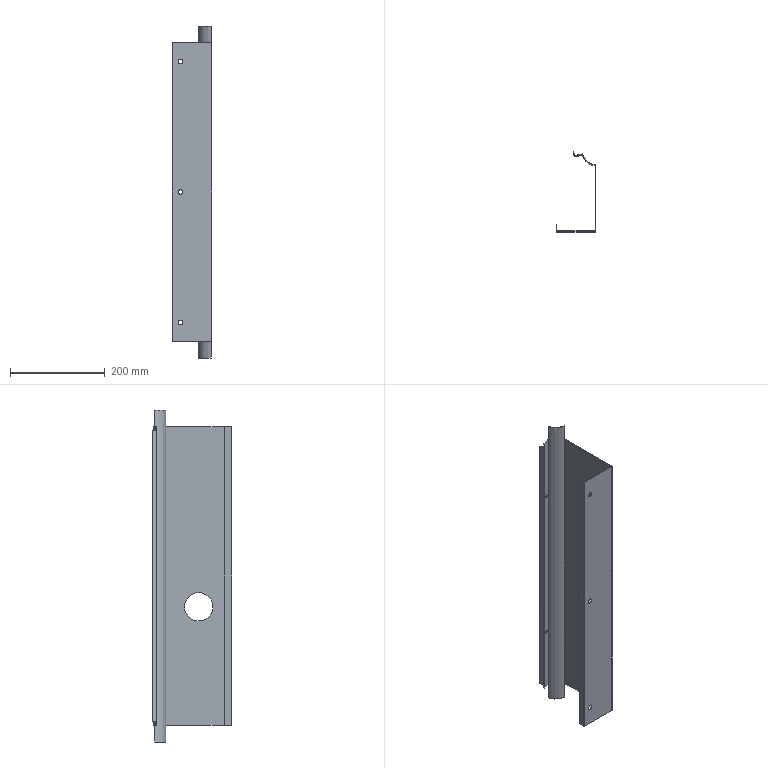Part | SolidWorks | features EdgeFlange 4, ICE 4, FlatPattern 1, SMBaseFlange 1, SheetMetal 1 | 1 solid | 57 faces | box 84 x 168.236 x 700 mm | volume 282210 mm3 | plane 38 | cylinder 19 | commonest cylinder face diameters 10 x6 3 x5 6 x4 60 x3 63 x1
STEP:
#1=CARTESIAN_POINT('',(0.,40.,-65.));
#2=VERTEX_POINT('',#1);
#3=CARTESIAN_POINT('',(0.,100.,-65.));
#4=VERTEX_POINT('',#3);
#5=CARTESIAN_POINT('',(0.,70.,-65.));
#6=DIRECTION('',(1.,0.,0.));
#7=DIRECTION('',(0.,1.,0.));
#8=AXIS2_PLACEMENT_3D('',#5,#6,#7);
#9=CIRCLE('',#8,30.);
#10=EDGE_CURVE('',#2,#4,#9,.T.);
#11=ORIENTED_EDGE('',*,*,#10,.F.);
#12=CARTESIAN_POINT('',(1.5,40.,-65.));
#13=VERTEX_POINT('',#12);
#14=CARTESIAN_POINT('',(0.,40.,-65.));
#15=DIRECTION('',(1.,0.,0.));
#16=VECTOR('',#15,1000.);
#17=LINE('',#14,#16);
#18=EDGE_CURVE('',#2,#13,#17,.T.);
#19=ORIENTED_EDGE('',*,*,#18,.T.);
#20=CARTESIAN_POINT('',(1.5,100.,-65.));
#21=VERTEX_POINT('',#20);
#22=CARTESIAN_POINT('',(1.5,70.,-65.));
#23=DIRECTION('',(1.,0.,0.));
#24=DIRECTION('',(0.,1.,0.));
#25=AXIS2_PLACEMENT_3D('',#22,#23,#24);
#26=CIRCLE('',#25,30.);
#27=EDGE_CURVE('',#13,#21,#26,.T.);
#28=ORIENTED_EDGE('',*,*,#27,.T.);
#29=CARTESIAN_POINT('',(0.,100.,-65.));
#30=DIRECTION('',(1.,0.,0.));
#31=VECTOR('',#30,1000.);
#32=LINE('',#29,#31);
#33=EDGE_CURVE('',#4,#21,#32,.T.);
#34=ORIENTED_EDGE('',*,*,#33,.F.);
#35=EDGE_LOOP('',(#11,#19,#28,#34));
#36=FACE_OUTER_BOUND('',#35,.T.);
#37=CARTESIAN_POINT('',(0.,70.,-65.));
#38=DIRECTION('',(1.,0.,0.));
#39=DIRECTION('',(0.,1.,0.));
#40=AXIS2_PLACEMENT_3D('',#37,#38,#39);
#41=CYLINDRICAL_SURFACE('',#40,30.);
#42=ADVANCED_FACE('',(#36),#41,.F.);
#43=CARTESIAN_POINT('',(-31.255,161.685,175.));
#44=VERTEX_POINT('',#43);
#45=CARTESIAN_POINT('',(-37.035,160.077,175.));
#46=VERTEX_POINT('',#45);
#47=CARTESIAN_POINT('',(-34.145,160.881,175.));
#48=DIRECTION('',(-0.268,0.9634,0.));
#49=DIRECTION('',(-0.9634,-0.268,0.));
#50=AXIS2_PLACEMENT_3D('',#47,#48,#49);
#51=CIRCLE('',#50,3.);
#52=EDGE_CURVE('',#44,#46,#51,.T.);
#53=ORIENTED_EDGE('',*,*,#52,.F.);
#54=CARTESIAN_POINT('',(-31.657,163.13,175.));
#55=VERTEX_POINT('',#54);
#56=CARTESIAN_POINT('',(-31.255,161.685,175.));
#57=DIRECTION('',(-0.268,0.9634,0.));
#58=VECTOR('',#57,1000.);
#59=LINE('',#56,#58);
#60=EDGE_CURVE('',#44,#55,#59,.T.);
#61=ORIENTED_EDGE('',*,*,#60,.T.);
#62=CARTESIAN_POINT('',(-37.437,161.522,175.));
#63=VERTEX_POINT('',#62);
#64=CARTESIAN_POINT('',(-34.547,162.326,175.));
#65=DIRECTION('',(-0.268,0.9634,0.));
#66=DIRECTION('',(-0.9634,-0.268,0.));
#67=AXIS2_PLACEMENT_3D('',#64,#65,#66);
#68=CIRCLE('',#67,3.);
#69=EDGE_CURVE('',#55,#63,#68,.T.);
#70=ORIENTED_EDGE('',*,*,#69,.T.);
#71=CARTESIAN_POINT('',(-37.035,160.077,175.));
#72=DIRECTION('',(-0.268,0.9634,0.));
#73=VECTOR('',#72,1000.);
#74=LINE('',#71,#73);
#75=EDGE_CURVE('',#46,#63,#74,.T.);
#76=ORIENTED_EDGE('',*,*,#75,.F.);
#77=EDGE_LOOP('',(#53,#61,#70,#76));
#78=FACE_OUTER_BOUND('',#77,.T.);
#79=CARTESIAN_POINT('',(-34.145,160.881,175.));
#80=DIRECTION('',(-0.268,0.9634,0.));
#81=DIRECTION('',(-0.9634,-0.268,0.));
#82=AXIS2_PLACEMENT_3D('',#79,#80,#81);
#83=CYLINDRICAL_SURFACE('',#82,3.);
#84=ADVANCED_FACE('',(#78),#83,.F.);
#85=CARTESIAN_POINT('',(-31.255,161.685,-175.));
#86=VERTEX_POINT('',#85);
#87=CARTESIAN_POINT('',(-37.035,160.077,-175.));
#88=VERTEX_POINT('',#87);
#89=CARTESIAN_POINT('',(-34.145,160.881,-175.));
#90=DIRECTION('',(-0.268,0.9634,0.));
#91=DIRECTION('',(-0.9634,-0.268,0.));
#92=AXIS2_PLACEMENT_3D('',#89,#90,#91);
#93=CIRCLE('',#92,3.);
#94=EDGE_CURVE('',#86,#88,#93,.T.);
#95=ORIENTED_EDGE('',*,*,#94,.F.);
#96=CARTESIAN_POINT('',(-31.657,163.13,-175.));
#97=VERTEX_POINT('',#96);
#98=CARTESIAN_POINT('',(-31.255,161.685,-175.));
#99=DIRECTION('',(-0.268,0.9634,0.));
#100=VECTOR('',#99,1000.);
#101=LINE('',#98,#100);
#102=EDGE_CURVE('',#86,#97,#101,.T.);
#103=ORIENTED_EDGE('',*,*,#102,.T.);
#104=CARTESIAN_POINT('',(-37.437,161.522,-175.));
#105=VERTEX_POINT('',#104);
#106=CARTESIAN_POINT('',(-34.547,162.326,-175.));
#107=DIRECTION('',(-0.268,0.9634,0.));
#108=DIRECTION('',(-0.9634,-0.268,0.));
#109=AXIS2_PLACEMENT_3D('',#106,#107,#108);
#110=CIRCLE('',#109,3.);
#111=EDGE_CURVE('',#97,#105,#110,.T.);
#112=ORIENTED_EDGE('',*,*,#111,.T.);
#113=CARTESIAN_POINT('',(-37.035,160.077,-175.));
#114=DIRECTION('',(-0.268,0.9634,0.));
#115=VECTOR('',#114,1000.);
#116=LINE('',#113,#115);
#117=EDGE_CURVE('',#88,#105,#116,.T.);
#118=ORIENTED_EDGE('',*,*,#117,.F.);
#119=EDGE_LOOP('',(#95,#103,#112,#118));
#120=FACE_OUTER_BOUND('',#119,.T.);
#121=CARTESIAN_POINT('',(-34.145,160.881,-175.));
#122=DIRECTION('',(-0.268,0.9634,0.));
#123=DIRECTION('',(-0.9634,-0.268,0.));
#124=AXIS2_PLACEMENT_3D('',#121,#122,#123);
#125=CYLINDRICAL_SURFACE('',#124,3.);
#126=ADVANCED_FACE('',(#120),#125,.F.);
#127=CARTESIAN_POINT('',(-70.,1.5,-275.));
#128=VERTEX_POINT('',#127);
#129=CARTESIAN_POINT('',(-60.,1.5,-275.));
#130=VERTEX_POINT('',#129);
#131=CARTESIAN_POINT('',(-65.,1.5,-275.));
#132=DIRECTION('',(0.,-1.,0.));
#133=DIRECTION('',(1.,0.,0.));
#134=AXIS2_PLACEMENT_3D('',#131,#132,#133);
#135=CIRCLE('',#134,5.);
#136=EDGE_CURVE('',#128,#130,#135,.T.);
#137=ORIENTED_EDGE('',*,*,#136,.F.);
#138=CARTESIAN_POINT('',(-70.,0.,-275.));
#139=VERTEX_POINT('',#138);
#140=CARTESIAN_POINT('',(-70.,1.5,-275.));
#141=DIRECTION('',(0.,-1.,0.));
#142=VECTOR('',#141,1000.);
#143=LINE('',#140,#142);
#144=EDGE_CURVE('',#128,#139,#143,.T.);
#145=ORIENTED_EDGE('',*,*,#144,.T.);
#146=CARTESIAN_POINT('',(-60.,0.,-275.));
#147=VERTEX_POINT('',#146);
#148=CARTESIAN_POINT('',(-65.,0.,-275.));
#149=DIRECTION('',(0.,-1.,0.));
#150=DIRECTION('',(1.,0.,0.));
#151=AXIS2_PLACEMENT_3D('',#148,#149,#150);
#152=CIRCLE('',#151,5.);
#153=EDGE_CURVE('',#139,#147,#152,.T.);
#154=ORIENTED_EDGE('',*,*,#153,.T.);
#155=CARTESIAN_POINT('',(-60.,1.5,-275.));
#156=DIRECTION('',(0.,-1.,0.));
#157=VECTOR('',#156,1000.);
#158=LINE('',#155,#157);
#159=EDGE_CURVE('',#130,#147,#158,.T.);
#160=ORIENTED_EDGE('',*,*,#159,.F.);
#161=EDGE_LOOP('',(#137,#145,#154,#160));
#162=FACE_OUTER_BOUND('',#161,.T.);
#163=CARTESIAN_POINT('',(-65.,1.5,-275.));
#164=DIRECTION('',(0.,-1.,0.));
#165=DIRECTION('',(1.,0.,0.));
#166=AXIS2_PLACEMENT_3D('',#163,#164,#165);
#167=CYLINDRICAL_SURFACE('',#166,5.);
#168=ADVANCED_FACE('',(#162),#167,.F.);
#169=CARTESIAN_POINT('',(-70.,1.5,0.));
#170=VERTEX_POINT('',#169);
#171=CARTESIAN_POINT('',(-60.,1.5,0.));
#172=VERTEX_POINT('',#171);
#173=CARTESIAN_POINT('',(-65.,1.5,0.));
#174=DIRECTION('',(0.,-1.,0.));
#175=DIRECTION('',(1.,0.,0.));
#176=AXIS2_PLACEMENT_3D('',#173,#174,#175);
#177=CIRCLE('',#176,5.);
#178=EDGE_CURVE('',#170,#172,#177,.T.);
#179=ORIENTED_EDGE('',*,*,#178,.F.);
#180=CARTESIAN_POINT('',(-70.,0.,0.));
#181=VERTEX_POINT('',#180);
#182=CARTESIAN_POINT('',(-70.,1.5,0.));
#183=DIRECTION('',(0.,-1.,0.));
#184=VECTOR('',#183,1000.);
#185=LINE('',#182,#184);
#186=EDGE_CURVE('',#170,#181,#185,.T.);
#187=ORIENTED_EDGE('',*,*,#186,.T.);
#188=CARTESIAN_POINT('',(-60.,0.,0.));
#189=VERTEX_POINT('',#188);
#190=CARTESIAN_POINT('',(-65.,0.,0.));
#191=DIRECTION('',(0.,-1.,0.));
#192=DIRECTION('',(1.,0.,0.));
#193=AXIS2_PLACEMENT_3D('',#190,#191,#192);
#194=CIRCLE('',#193,5.);
#195=EDGE_CURVE('',#181,#189,#194,.T.);
#196=ORIENTED_EDGE('',*,*,#195,.T.);
#197=CARTESIAN_POINT('',(-60.,1.5,0.));
#198=DIRECTION('',(0.,-1.,0.));
#199=VECTOR('',#198,1000.);
#200=LINE('',#197,#199);
#201=EDGE_CURVE('',#172,#189,#200,.T.);
#202=ORIENTED_EDGE('',*,*,#201,.F.);
#203=EDGE_LOOP('',(#179,#187,#196,#202));
#204=FACE_OUTER_BOUND('',#203,.T.);
#205=CARTESIAN_POINT('',(-65.,1.5,0.));
#206=DIRECTION('',(0.,-1.,0.));
#207=DIRECTION('',(1.,0.,0.));
#208=AXIS2_PLACEMENT_3D('',#205,#206,#207);
#209=CYLINDRICAL_SURFACE('',#208,5.);
#210=ADVANCED_FACE('',(#204),#209,.F.);
#211=CARTESIAN_POINT('',(-70.,1.5,275.));
#212=VERTEX_POINT('',#211);
#213=CARTESIAN_POINT('',(-60.,1.5,275.));
#214=VERTEX_POINT('',#213);
#215=CARTESIAN_POINT('',(-65.,1.5,275.));
#216=DIRECTION('',(0.,-1.,0.));
#217=DIRECTION('',(1.,0.,0.));
#218=AXIS2_PLACEMENT_3D('',#215,#216,#217);
#219=CIRCLE('',#218,5.);
#220=EDGE_CURVE('',#212,#214,#219,.T.);
#221=ORIENTED_EDGE('',*,*,#220,.F.);
#222=CARTESIAN_POINT('',(-70.,0.,275.));
#223=VERTEX_POINT('',#222);
#224=CARTESIAN_POINT('',(-70.,1.5,275.));
#225=DIRECTION('',(0.,-1.,0.));
#226=VECTOR('',#225,1000.);
#227=LINE('',#224,#226);
#228=EDGE_CURVE('',#212,#223,#227,.T.);
#229=ORIENTED_EDGE('',*,*,#228,.T.);
#230=CARTESIAN_POINT('',(-60.,0.,275.));
#231=VERTEX_POINT('',#230);
#232=CARTESIAN_POINT('',(-65.,0.,275.));
#233=DIRECTION('',(0.,-1.,0.));
#234=DIRECTION('',(1.,0.,0.));
#235=AXIS2_PLACEMENT_3D('',#232,#233,#234);
#236=CIRCLE('',#235,5.);
#237=EDGE_CURVE('',#223,#231,#236,.T.);
#238=ORIENTED_EDGE('',*,*,#237,.T.);
#239=CARTESIAN_POINT('',(-60.,1.5,275.));
#240=DIRECTION('',(0.,-1.,0.));
#241=VECTOR('',#240,1000.);
#242=LINE('',#239,#241);
#243=EDGE_CURVE('',#214,#231,#242,.T.);
#244=ORIENTED_EDGE('',*,*,#243,.F.);
#245=EDGE_LOOP('',(#221,#229,#238,#244));
#246=FACE_OUTER_BOUND('',#245,.T.);
#247=CARTESIAN_POINT('',(-65.,1.5,275.));
#248=DIRECTION('',(0.,-1.,0.));
#249=DIRECTION('',(1.,0.,0.));
#250=AXIS2_PLACEMENT_3D('',#247,#248,#249);
#251=CYLINDRICAL_SURFACE('',#250,5.);
#252=ADVANCED_FACE('',(#246),#251,.F.);
#253=CARTESIAN_POINT('',(-81.,1.5,315.));
#254=VERTEX_POINT('',#253);
#255=CARTESIAN_POINT('',(0.,1.5,315.));
#256=VERTEX_POINT('',#255);
#257=CARTESIAN_POINT('',(0.,1.5,315.));
#258=DIRECTION('',(1.,0.,0.));
#259=VECTOR('',#258,1000.);
#260=LINE('',#257,#259);
#261=EDGE_CURVE('',#254,#256,#260,.T.);
#262=ORIENTED_EDGE('',*,*,#261,.F.);
#263=CARTESIAN_POINT('',(-81.,0.,315.));
#264=VERTEX_POINT('',#263);
#265=CARTESIAN_POINT('',(-81.,0.,315.));
#266=DIRECTION('',(0.,1.,0.));
#267=VECTOR('',#266,1000.);
#268=LINE('',#265,#267);
#269=EDGE_CURVE('',#264,#254,#268,.T.);
#270=ORIENTED_EDGE('',*,*,#269,.F.);
#271=CARTESIAN_POINT('',(0.,0.,315.));
#272=VERTEX_POINT('',#271);
#273=CARTESIAN_POINT('',(0.,0.,315.));
#274=DIRECTION('',(1.,0.,0.));
#275=VECTOR('',#274,1000.);
#276=LINE('',#273,#275);
#277=EDGE_CURVE('',#264,#272,#276,.T.);
#278=ORIENTED_EDGE('',*,*,#277,.T.);
#279=CARTESIAN_POINT('',(0.,0.,315.));
#280=DIRECTION('',(0.,1.,0.));
#281=VECTOR('',#280,1000.);
#282=LINE('',#279,#281);
#283=EDGE_CURVE('',#272,#256,#282,.T.);
#284=ORIENTED_EDGE('',*,*,#283,.T.);
#285=EDGE_LOOP('',(#262,#270,#278,#284));
#286=FACE_OUTER_BOUND('',#285,.T.);
#287=CARTESIAN_POINT('',(0.,0.,315.));
#288=DIRECTION('',(0.,0.,1.));
#289=DIRECTION('',(0.,-1.,0.));
#290=AXIS2_PLACEMENT_3D('',#287,#288,#289);
#291=PLANE('',#290);
#292=ADVANCED_FACE('',(#286),#291,.T.);
#293=CARTESIAN_POINT('',(-65.,0.,-275.));
#294=DIRECTION('',(0.,-1.,0.));
#295=DIRECTION('',(1.,0.,0.));
#296=AXIS2_PLACEMENT_3D('',#293,#294,#295);
#297=CIRCLE('',#296,5.);
#298=EDGE_CURVE('',#147,#139,#297,.T.);
#299=ORIENTED_EDGE('',*,*,#298,.F.);
#300=ORIENTED_EDGE('',*,*,#153,.F.);
#301=EDGE_LOOP('',(#299,#300));
#302=FACE_BOUND('',#301,.T.);
#303=CARTESIAN_POINT('',(-65.,0.,0.));
#304=DIRECTION('',(0.,-1.,0.));
#305=DIRECTION('',(1.,0.,0.));
#306=AXIS2_PLACEMENT_3D('',#303,#304,#305);
#307=CIRCLE('',#306,5.);
#308=EDGE_CURVE('',#189,#181,#307,.T.);
#309=ORIENTED_EDGE('',*,*,#308,.F.);
#310=ORIENTED_EDGE('',*,*,#195,.F.);
#311=EDGE_LOOP('',(#309,#310));
#312=FACE_BOUND('',#311,.T.);
#313=CARTESIAN_POINT('',(-65.,0.,275.));
#314=DIRECTION('',(0.,-1.,0.));
#315=DIRECTION('',(1.,0.,0.));
#316=AXIS2_PLACEMENT_3D('',#313,#314,#315);
#317=CIRCLE('',#316,5.);
#318=EDGE_CURVE('',#231,#223,#317,.T.);
#319=ORIENTED_EDGE('',*,*,#318,.F.);
#320=ORIENTED_EDGE('',*,*,#237,.F.);
#321=EDGE_LOOP('',(#319,#320));
#322=FACE_BOUND('',#321,.T.);
#323=ORIENTED_EDGE('',*,*,#277,.F.);
#324=CARTESIAN_POINT('',(-81.,0.,-315.));
#325=VERTEX_POINT('',#324);
#326=CARTESIAN_POINT('',(-81.,0.,315.));
#327=DIRECTION('',(0.,0.,1.));
#328=VECTOR('',#327,1000.);
#329=LINE('',#326,#328);
#330=EDGE_CURVE('',#325,#264,#329,.T.);
#331=ORIENTED_EDGE('',*,*,#330,.F.);
#332=CARTESIAN_POINT('',(0.,0.,-315.));
#333=VERTEX_POINT('',#332);
#334=CARTESIAN_POINT('',(-82.5,0.,-315.));
#335=DIRECTION('',(-1.,0.,0.));
#336=VECTOR('',#335,1000.);
#337=LINE('',#334,#336);
#338=EDGE_CURVE('',#333,#325,#337,.T.);
#339=ORIENTED_EDGE('',*,*,#338,.F.);
#340=CARTESIAN_POINT('',(0.,0.,-315.));
#341=DIRECTION('',(0.,0.,-1.));
#342=VECTOR('',#341,1000.);
#343=LINE('',#340,#342);
#344=EDGE_CURVE('',#272,#333,#343,.T.);
#345=ORIENTED_EDGE('',*,*,#344,.F.);
#346=EDGE_LOOP('',(#323,#331,#339,#345));
#347=FACE_OUTER_BOUND('',#346,.T.);
#348=CARTESIAN_POINT('',(0.,0.,315.));
#349=DIRECTION('',(0.,-1.,0.));
#350=DIRECTION('',(1.,0.,0.));
#351=AXIS2_PLACEMENT_3D('',#348,#349,#350);
#352=PLANE('',#351);
#353=ADVANCED_FACE('',(#302,#312,#322,#347),#352,.T.);
#354=CARTESIAN_POINT('',(-65.,1.5,-275.));
#355=DIRECTION('',(0.,-1.,0.));
#356=DIRECTION('',(1.,0.,0.));
#357=AXIS2_PLACEMENT_3D('',#354,#355,#356);
#358=CIRCLE('',#357,5.);
#359=EDGE_CURVE('',#130,#128,#358,.T.);
#360=ORIENTED_EDGE('',*,*,#359,.T.);
#361=ORIENTED_EDGE('',*,*,#136,.T.);
#362=EDGE_LOOP('',(#360,#361));
#363=FACE_BOUND('',#362,.T.);
#364=CARTESIAN_POINT('',(-65.,1.5,0.));
#365=DIRECTION('',(0.,-1.,0.));
#366=DIRECTION('',(1.,0.,0.));
#367=AXIS2_PLACEMENT_3D('',#364,#365,#366);
#368=CIRCLE('',#367,5.);
#369=EDGE_CURVE('',#172,#170,#368,.T.);
#370=ORIENTED_EDGE('',*,*,#369,.T.);
#371=ORIENTED_EDGE('',*,*,#178,.T.);
#372=EDGE_LOOP('',(#370,#371));
#373=FACE_BOUND('',#372,.T.);
#374=CARTESIAN_POINT('',(-65.,1.5,275.));
#375=DIRECTION('',(0.,-1.,0.));
#376=DIRECTION('',(1.,0.,0.));
#377=AXIS2_PLACEMENT_3D('',#374,#375,#376);
#378=CIRCLE('',#377,5.);
#379=EDGE_CURVE('',#214,#212,#378,.T.);
#380=ORIENTED_EDGE('',*,*,#379,.T.);
#381=ORIENTED_EDGE('',*,*,#220,.T.);
#382=EDGE_LOOP('',(#380,#381));
#383=FACE_BOUND('',#382,.T.);
#384=CARTESIAN_POINT('',(-81.,1.5,-315.));
#385=VERTEX_POINT('',#384);
#386=CARTESIAN_POINT('',(-81.,1.5,-315.));
#387=DIRECTION('',(0.,0.,1.));
#388=VECTOR('',#387,1000.);
#389=LINE('',#386,#388);
#390=EDGE_CURVE('',#385,#254,#389,.T.);
#391=ORIENTED_EDGE('',*,*,#390,.T.);
#392=ORIENTED_EDGE('',*,*,#261,.T.);
#393=CARTESIAN_POINT('',(0.,1.5,-315.));
#394=VERTEX_POINT('',#393);
#395=CARTESIAN_POINT('',(0.,1.5,315.));
#396=DIRECTION('',(0.,0.,-1.));
#397=VECTOR('',#396,1000.);
#398=LINE('',#395,#397);
#399=EDGE_CURVE('',#256,#394,#398,.T.);
#400=ORIENTED_EDGE('',*,*,#399,.T.);
#401=CARTESIAN_POINT('',(0.,1.5,-315.));
#402=DIRECTION('',(-1.,0.,0.));
#403=VECTOR('',#402,1000.);
#404=LINE('',#401,#403);
#405=EDGE_CURVE('',#394,#385,#404,.T.);
#406=ORIENTED_EDGE('',*,*,#405,.T.);
#407=EDGE_LOOP('',(#391,#392,#400,#406));
#408=FACE_OUTER_BOUND('',#407,.T.);
#409=CARTESIAN_POINT('',(0.,1.5,315.));
#410=DIRECTION('',(0.,-1.,0.));
#411=DIRECTION('',(1.,0.,0.));
#412=AXIS2_PLACEMENT_3D('',#409,#410,#411);
#413=PLANE('',#412);
#414=ADVANCED_FACE('',(#363,#373,#383,#408),#413,.F.);
#415=CARTESIAN_POINT('',(0.,70.,-65.));
#416=DIRECTION('',(1.,0.,0.));
#417=DIRECTION('',(0.,1.,0.));
#418=AXIS2_PLACEMENT_3D('',#415,#416,#417);
#419=CIRCLE('',#418,30.);
#420=EDGE_CURVE('',#4,#2,#419,.T.);
#421=ORIENTED_EDGE('',*,*,#420,.T.);
#422=ORIENTED_EDGE('',*,*,#10,.T.);
#423=EDGE_LOOP('',(#421,#422));
#424=FACE_BOUND('',#423,.T.);
#425=CARTESIAN_POINT('',(0.,139.838,-315.));
#426=VERTEX_POINT('',#425);
#427=CARTESIAN_POINT('',(0.,214.203,-315.));
#428=DIRECTION('',(0.,-1.,0.));
#429=VECTOR('',#428,1000.);
#430=LINE('',#427,#429);
#431=EDGE_CURVE('',#426,#394,#430,.T.);
#432=ORIENTED_EDGE('',*,*,#431,.T.);
#433=ORIENTED_EDGE('',*,*,#399,.F.);
#434=CARTESIAN_POINT('',(0.,139.838,315.));
#435=VERTEX_POINT('',#434);
#436=CARTESIAN_POINT('',(0.,208.924,315.));
#437=DIRECTION('',(0.,1.,0.));
#438=VECTOR('',#437,1000.);
#439=LINE('',#436,#438);
#440=EDGE_CURVE('',#256,#435,#439,.T.);
#441=ORIENTED_EDGE('',*,*,#440,.T.);
#442=CARTESIAN_POINT('',(0.,139.838,350.));
#443=DIRECTION('',(0.,0.,-1.));
#444=VECTOR('',#443,1000.);
#445=LINE('',#442,#444);
#446=EDGE_CURVE('',#435,#426,#445,.T.);
#447=ORIENTED_EDGE('',*,*,#446,.T.);
#448=EDGE_LOOP('',(#432,#433,#441,#447));
#449=FACE_OUTER_BOUND('',#448,.T.);
#450=CARTESIAN_POINT('',(0.,0.,350.));
#451=DIRECTION('',(-1.,0.,0.));
#452=DIRECTION('',(0.,-1.,0.));
#453=AXIS2_PLACEMENT_3D('',#450,#451,#452);
#454=PLANE('',#453);
#455=ADVANCED_FACE('',(#424,#449),#454,.T.);
#456=CARTESIAN_POINT('',(1.5,70.,-65.));
#457=DIRECTION('',(1.,0.,0.));
#458=DIRECTION('',(0.,1.,0.));
#459=AXIS2_PLACEMENT_3D('',#456,#457,#458);
#460=CIRCLE('',#459,30.);
#461=EDGE_CURVE('',#21,#13,#460,.T.);
#462=ORIENTED_EDGE('',*,*,#461,.F.);
#463=ORIENTED_EDGE('',*,*,#27,.F.);
#464=EDGE_LOOP('',(#462,#463));
#465=FACE_BOUND('',#464,.T.);
#466=CARTESIAN_POINT('',(1.5,1.5,315.));
#467=VERTEX_POINT('',#466);
#468=CARTESIAN_POINT('',(1.5,1.5,-315.));
#469=VERTEX_POINT('',#468);
#470=CARTESIAN_POINT('',(1.5,1.5,-315.));
#471=DIRECTION('',(0.,0.,-1.));
#472=VECTOR('',#471,1000.);
#473=LINE('',#470,#472);
#474=EDGE_CURVE('',#467,#469,#473,.T.);
#475=ORIENTED_EDGE('',*,*,#474,.T.);
#476=CARTESIAN_POINT('',(1.5,139.838,-315.));
#477=VERTEX_POINT('',#476);
#478=CARTESIAN_POINT('',(1.5,214.203,-315.));
#479=DIRECTION('',(0.,-1.,0.));
#480=VECTOR('',#479,1000.);
#481=LINE('',#478,#480);
#482=EDGE_CURVE('',#477,#469,#481,.T.);
#483=ORIENTED_EDGE('',*,*,#482,.F.);
#484=CARTESIAN_POINT('',(1.5,139.838,315.));
#485=VERTEX_POINT('',#484);
#486=CARTESIAN_POINT('',(1.5,139.838,350.));
#487=DIRECTION('',(0.,0.,1.));
#488=VECTOR('',#487,1000.);
#489=LINE('',#486,#488);
#490=EDGE_CURVE('',#477,#485,#489,.T.);
#491=ORIENTED_EDGE('',*,*,#490,.T.);
#492=CARTESIAN_POINT('',(1.5,208.924,315.));
#493=DIRECTION('',(0.,1.,0.));
#494=VECTOR('',#493,1000.);
#495=LINE('',#492,#494);
#496=EDGE_CURVE('',#467,#485,#495,.T.);
#497=ORIENTED_EDGE('',*,*,#496,.F.);
#498=EDGE_LOOP('',(#475,#483,#491,#497));
#499=FACE_OUTER_BOUND('',#498,.T.);
#500=CARTESIAN_POINT('',(1.5,0.,350.));
#501=DIRECTION('',(-1.,0.,0.));
#502=DIRECTION('',(0.,-1.,0.));
#503=AXIS2_PLACEMENT_3D('',#500,#501,#502);
#504=PLANE('',#503);
#505=ADVANCED_FACE('',(#465,#499),#504,.F.);
#506=CARTESIAN_POINT('',(1.5,1.5,315.));
#507=DIRECTION('',(-1.,0.,0.));
#508=VECTOR('',#507,1000.);
#509=LINE('',#506,#508);
#510=EDGE_CURVE('',#467,#256,#509,.T.);
#511=ORIENTED_EDGE('',*,*,#510,.F.);
#512=ORIENTED_EDGE('',*,*,#496,.T.);
#513=CARTESIAN_POINT('',(0.1403,141.331,315.));
#514=VERTEX_POINT('',#513);
#515=CARTESIAN_POINT('',(0.,139.838,315.));
#516=DIRECTION('',(0.,0.,1.));
#517=DIRECTION('',(-1.,0.,0.));
#518=AXIS2_PLACEMENT_3D('',#515,#516,#517);
#519=CIRCLE('',#518,1.5);
#520=EDGE_CURVE('',#485,#514,#519,.T.);
#521=ORIENTED_EDGE('',*,*,#520,.T.);
#522=CARTESIAN_POINT('',(0.,141.345,315.));
#523=VERTEX_POINT('',#522);
#524=CARTESIAN_POINT('',(2.946,171.2,315.));
#525=DIRECTION('',(0.,0.,1.));
#526=DIRECTION('',(-1.,0.,0.));
#527=AXIS2_PLACEMENT_3D('',#524,#525,#526);
#528=CIRCLE('',#527,30.);
#529=EDGE_CURVE('',#523,#514,#528,.T.);
#530=ORIENTED_EDGE('',*,*,#529,.F.);
#531=CARTESIAN_POINT('',(0.,208.924,315.));
#532=DIRECTION('',(0.,1.,0.));
#533=VECTOR('',#532,1000.);
#534=LINE('',#531,#533);
#535=EDGE_CURVE('',#435,#523,#534,.T.);
#536=ORIENTED_EDGE('',*,*,#535,.F.);
#537=ORIENTED_EDGE('',*,*,#440,.F.);
#538=EDGE_LOOP('',(#511,#512,#521,#530,#536,#537));
#539=FACE_OUTER_BOUND('',#538,.T.);
#540=CARTESIAN_POINT('',(0.,208.924,315.));
#541=DIRECTION('',(0.,0.,-1.));
#542=DIRECTION('',(-1.,0.,0.));
#543=AXIS2_PLACEMENT_3D('',#540,#541,#542);
#544=PLANE('',#543);
#545=ADVANCED_FACE('',(#539),#544,.F.);
#546=CARTESIAN_POINT('',(1.5,1.5,-315.));
#547=DIRECTION('',(-1.,0.,0.));
#548=VECTOR('',#547,1000.);
#549=LINE('',#546,#548);
#550=EDGE_CURVE('',#469,#394,#549,.T.);
#551=ORIENTED_EDGE('',*,*,#550,.T.);
#552=ORIENTED_EDGE('',*,*,#431,.F.);
#553=CARTESIAN_POINT('',(0.,141.345,-315.));
#554=VERTEX_POINT('',#553);
#555=CARTESIAN_POINT('',(0.,214.203,-315.));
#556=DIRECTION('',(0.,-1.,0.));
#557=VECTOR('',#556,1000.);
#558=LINE('',#555,#557);
#559=EDGE_CURVE('',#554,#426,#558,.T.);
#560=ORIENTED_EDGE('',*,*,#559,.F.);
#561=CARTESIAN_POINT('',(0.1403,141.331,-315.));
#562=VERTEX_POINT('',#561);
#563=CARTESIAN_POINT('',(2.946,171.2,-315.));
#564=DIRECTION('',(0.,0.,-1.));
#565=DIRECTION('',(1.,0.,0.));
#566=AXIS2_PLACEMENT_3D('',#563,#564,#565);
#567=CIRCLE('',#566,30.);
#568=EDGE_CURVE('',#562,#554,#567,.T.);
#569=ORIENTED_EDGE('',*,*,#568,.F.);
#570=CARTESIAN_POINT('',(0.,139.838,-315.));
#571=DIRECTION('',(0.,0.,-1.));
#572=DIRECTION('',(1.,0.,0.));
#573=AXIS2_PLACEMENT_3D('',#570,#571,#572);
#574=CIRCLE('',#573,1.5);
#575=EDGE_CURVE('',#562,#477,#574,.T.);
#576=ORIENTED_EDGE('',*,*,#575,.T.);
#577=ORIENTED_EDGE('',*,*,#482,.T.);
#578=EDGE_LOOP('',(#551,#552,#560,#569,#576,#577));
#579=FACE_OUTER_BOUND('',#578,.T.);
#580=CARTESIAN_POINT('',(0.,214.203,-315.));
#581=DIRECTION('',(0.,0.,1.));
#582=DIRECTION('',(1.,0.,0.));
#583=AXIS2_PLACEMENT_3D('',#580,#581,#582);
#584=PLANE('',#583);
#585=ADVANCED_FACE('',(#579),#584,.F.);
#586=CARTESIAN_POINT('',(-42.334,158.602,-306.5));
#587=VERTEX_POINT('',#586);
#588=CARTESIAN_POINT('',(-42.334,158.602,-315.));
#589=VERTEX_POINT('',#588);
#590=CARTESIAN_POINT('',(-42.334,158.602,-315.));
#591=DIRECTION('',(0.,0.,-1.));
#592=VECTOR('',#591,1000.);
#593=LINE('',#590,#592);
#594=EDGE_CURVE('',#587,#589,#593,.T.);
#595=ORIENTED_EDGE('',*,*,#594,.F.);
#596=CARTESIAN_POINT('',(-42.736,160.047,-306.5));
#597=VERTEX_POINT('',#596);
#598=CARTESIAN_POINT('',(-42.334,158.602,-306.5));
#599=DIRECTION('',(-0.268,0.9634,0.));
#600=VECTOR('',#599,1000.);
#601=LINE('',#598,#600);
#602=EDGE_CURVE('',#587,#597,#601,.T.);
#603=ORIENTED_EDGE('',*,*,#602,.T.);
#604=CARTESIAN_POINT('',(-42.736,160.047,-315.));
#605=VERTEX_POINT('',#604);
#606=CARTESIAN_POINT('',(-42.736,160.047,-315.));
#607=DIRECTION('',(0.,0.,-1.));
#608=VECTOR('',#607,1000.);
#609=LINE('',#606,#608);
#610=EDGE_CURVE('',#597,#605,#609,.T.);
#611=ORIENTED_EDGE('',*,*,#610,.T.);
#612=CARTESIAN_POINT('',(-42.736,160.047,-315.));
#613=DIRECTION('',(0.268,-0.9634,0.));
#614=VECTOR('',#613,1000.);
#615=LINE('',#612,#614);
#616=EDGE_CURVE('',#605,#589,#615,.T.);
#617=ORIENTED_EDGE('',*,*,#616,.T.);
#618=EDGE_LOOP('',(#595,#603,#611,#617));
#619=FACE_OUTER_BOUND('',#618,.T.);
#620=CARTESIAN_POINT('',(-42.736,160.047,-315.));
#621=DIRECTION('',(-0.9634,-0.268,0.));
#622=DIRECTION('',(0.268,-0.9634,0.));
#623=AXIS2_PLACEMENT_3D('',#620,#621,#622);
#624=PLANE('',#623);
#625=ADVANCED_FACE('',(#619),#624,.T.);
#626=CARTESIAN_POINT('',(-25.956,163.159,350.));
#627=VERTEX_POINT('',#626);
#628=CARTESIAN_POINT('',(-25.956,163.159,315.));
#629=VERTEX_POINT('',#628);
#630=CARTESIAN_POINT('',(-25.956,163.159,350.));
#631=DIRECTION('',(0.,0.,-1.));
#632=VECTOR('',#631,1000.);
#633=LINE('',#630,#632);
#634=EDGE_CURVE('',#627,#629,#633,.T.);
#635=ORIENTED_EDGE('',*,*,#634,.T.);
#636=CARTESIAN_POINT('',(-27.401,162.757,315.));
#637=VERTEX_POINT('',#636);
#638=CARTESIAN_POINT('',(-25.956,163.159,315.));
#639=DIRECTION('',(-0.9634,-0.268,0.));
#640=VECTOR('',#639,1000.);
#641=LINE('',#638,#640);
#642=EDGE_CURVE('',#629,#637,#641,.T.);
#643=ORIENTED_EDGE('',*,*,#642,.T.);
#644=CARTESIAN_POINT('',(-27.401,162.757,350.));
#645=VERTEX_POINT('',#644);
#646=CARTESIAN_POINT('',(-27.401,162.757,350.));
#647=DIRECTION('',(0.,0.,-1.));
#648=VECTOR('',#647,1000.);
#649=LINE('',#646,#648);
#650=EDGE_CURVE('',#645,#637,#649,.T.);
#651=ORIENTED_EDGE('',*,*,#650,.F.);
#652=CARTESIAN_POINT('',(-27.401,162.757,350.));
#653=DIRECTION('',(0.9634,0.268,0.));
#654=VECTOR('',#653,1000.);
#655=LINE('',#652,#654);
#656=EDGE_CURVE('',#645,#627,#655,.T.);
#657=ORIENTED_EDGE('',*,*,#656,.T.);
#658=EDGE_LOOP('',(#635,#643,#651,#657));
#659=FACE_OUTER_BOUND('',#658,.T.);
#660=CARTESIAN_POINT('',(-27.401,162.757,350.));
#661=DIRECTION('',(-0.268,0.9634,0.));
#662=DIRECTION('',(-0.9634,-0.268,0.));
#663=AXIS2_PLACEMENT_3D('',#660,#661,#662);
#664=PLANE('',#663);
#665=ADVANCED_FACE('',(#659),#664,.T.);
#666=CARTESIAN_POINT('',(0.,141.345,-350.));
#667=VERTEX_POINT('',#666);
#668=CARTESIAN_POINT('',(-25.956,163.159,-350.));
#669=VERTEX_POINT('',#668);
#670=CARTESIAN_POINT('',(2.946,171.2,-350.));
#671=DIRECTION('',(0.,0.,-1.));
#672=DIRECTION('',(1.,0.,0.));
#673=AXIS2_PLACEMENT_3D('',#670,#671,#672);
#674=CIRCLE('',#673,30.);
#675=EDGE_CURVE('',#667,#669,#674,.T.);
#676=ORIENTED_EDGE('',*,*,#675,.F.);
#677=CARTESIAN_POINT('',(0.,139.838,-350.));
#678=VERTEX_POINT('',#677);
#679=CARTESIAN_POINT('',(0.,214.203,-350.));
#680=DIRECTION('',(0.,1.,0.));
#681=VECTOR('',#680,1000.);
#682=LINE('',#679,#681);
#683=EDGE_CURVE('',#678,#667,#682,.T.);
#684=ORIENTED_EDGE('',*,*,#683,.F.);
#685=CARTESIAN_POINT('',(-27.401,162.757,-350.));
#686=VERTEX_POINT('',#685);
#687=CARTESIAN_POINT('',(2.946,171.2,-350.));
#688=DIRECTION('',(0.,0.,-1.));
#689=DIRECTION('',(1.,0.,0.));
#690=AXIS2_PLACEMENT_3D('',#687,#688,#689);
#691=CIRCLE('',#690,31.5);
#692=EDGE_CURVE('',#678,#686,#691,.T.);
#693=ORIENTED_EDGE('',*,*,#692,.T.);
#694=CARTESIAN_POINT('',(-27.401,162.757,-350.));
#695=DIRECTION('',(0.9634,0.268,0.));
#696=VECTOR('',#695,1000.);
#697=LINE('',#694,#696);
#698=EDGE_CURVE('',#686,#669,#697,.T.);
#699=ORIENTED_EDGE('',*,*,#698,.T.);
#700=EDGE_LOOP('',(#676,#684,#693,#699));
#701=FACE_OUTER_BOUND('',#700,.T.);
#702=CARTESIAN_POINT('',(0.,139.838,-350.));
#703=DIRECTION('',(0.,0.,-1.));
#704=DIRECTION('',(-1.,0.,0.));
#705=AXIS2_PLACEMENT_3D('',#702,#703,#704);
#706=PLANE('',#705);
#707=ADVANCED_FACE('',(#701),#706,.T.);
#708=CARTESIAN_POINT('',(0.1403,141.331,350.));
#709=DIRECTION('',(0.,0.,-1.));
#710=VECTOR('',#709,1000.);
#711=LINE('',#708,#710);
#712=EDGE_CURVE('',#514,#562,#711,.T.);
#713=ORIENTED_EDGE('',*,*,#712,.T.);
#714=ORIENTED_EDGE('',*,*,#568,.T.);
#715=CARTESIAN_POINT('',(0.,141.345,350.));
#716=DIRECTION('',(0.,0.,1.));
#717=VECTOR('',#716,1000.);
#718=LINE('',#715,#717);
#719=EDGE_CURVE('',#667,#554,#718,.T.);
#720=ORIENTED_EDGE('',*,*,#719,.F.);
#721=ORIENTED_EDGE('',*,*,#675,.T.);
#722=CARTESIAN_POINT('',(-25.956,163.159,-315.));
#723=VERTEX_POINT('',#722);
#724=CARTESIAN_POINT('',(-25.956,163.159,350.));
#725=DIRECTION('',(0.,0.,-1.));
#726=VECTOR('',#725,1000.);
#727=LINE('',#724,#726);
#728=EDGE_CURVE('',#723,#669,#727,.T.);
#729=ORIENTED_EDGE('',*,*,#728,.F.);
#730=CARTESIAN_POINT('',(-25.956,163.159,315.));
#731=DIRECTION('',(0.,0.,1.));
#732=VECTOR('',#731,1000.);
#733=LINE('',#730,#732);
#734=EDGE_CURVE('',#723,#629,#733,.T.);
#735=ORIENTED_EDGE('',*,*,#734,.T.);
#736=ORIENTED_EDGE('',*,*,#634,.F.);
#737=CARTESIAN_POINT('',(0.,141.345,350.));
#738=VERTEX_POINT('',#737);
#739=CARTESIAN_POINT('',(2.946,171.2,350.));
#740=DIRECTION('',(0.,0.,-1.));
#741=DIRECTION('',(1.,0.,0.));
#742=AXIS2_PLACEMENT_3D('',#739,#740,#741);
#743=CIRCLE('',#742,30.);
#744=EDGE_CURVE('',#738,#627,#743,.T.);
#745=ORIENTED_EDGE('',*,*,#744,.F.);
#746=CARTESIAN_POINT('',(0.,141.345,350.));
#747=DIRECTION('',(0.,0.,-1.));
#748=VECTOR('',#747,1000.);
#749=LINE('',#746,#748);
#750=EDGE_CURVE('',#738,#523,#749,.T.);
#751=ORIENTED_EDGE('',*,*,#750,.T.);
#752=ORIENTED_EDGE('',*,*,#529,.T.);
#753=EDGE_LOOP('',(#713,#714,#720,#721,#729,#735,#736,#745,#751,#752));
#754=FACE_OUTER_BOUND('',#753,.T.);
#755=CARTESIAN_POINT('',(2.946,171.2,350.));
#756=DIRECTION('',(0.,0.,-1.));
#757=DIRECTION('',(-1.,0.,0.));
#758=AXIS2_PLACEMENT_3D('',#755,#756,#757);
#759=CYLINDRICAL_SURFACE('',#758,30.);
#760=ADVANCED_FACE('',(#754),#759,.F.);
#761=CARTESIAN_POINT('',(-27.401,162.757,-315.));
#762=VERTEX_POINT('',#761);
#763=CARTESIAN_POINT('',(-25.956,163.159,-315.));
#764=DIRECTION('',(-0.9634,-0.268,0.));
#765=VECTOR('',#764,1000.);
#766=LINE('',#763,#765);
#767=EDGE_CURVE('',#723,#762,#766,.T.);
#768=ORIENTED_EDGE('',*,*,#767,.F.);
#769=ORIENTED_EDGE('',*,*,#728,.T.);
#770=ORIENTED_EDGE('',*,*,#698,.F.);
#771=CARTESIAN_POINT('',(-27.401,162.757,350.));
#772=DIRECTION('',(0.,0.,-1.));
#773=VECTOR('',#772,1000.);
#774=LINE('',#771,#773);
#775=EDGE_CURVE('',#762,#686,#774,.T.);
#776=ORIENTED_EDGE('',*,*,#775,.F.);
#777=EDGE_LOOP('',(#768,#769,#770,#776));
#778=FACE_OUTER_BOUND('',#777,.T.);
#779=CARTESIAN_POINT('',(-27.401,162.757,350.));
#780=DIRECTION('',(-0.268,0.9634,0.));
#781=DIRECTION('',(-0.9634,-0.268,0.));
#782=AXIS2_PLACEMENT_3D('',#779,#780,#781);
#783=PLANE('',#782);
#784=ADVANCED_FACE('',(#778),#783,.T.);
#785=ORIENTED_EDGE('',*,*,#692,.F.);
#786=CARTESIAN_POINT('',(0.,139.838,350.));
#787=DIRECTION('',(0.,0.,1.));
#788=VECTOR('',#787,1000.);
#789=LINE('',#786,#788);
#790=EDGE_CURVE('',#678,#426,#789,.T.);
#791=ORIENTED_EDGE('',*,*,#790,.T.);
#792=ORIENTED_EDGE('',*,*,#446,.F.);
#793=CARTESIAN_POINT('',(0.,139.838,350.));
#794=VERTEX_POINT('',#793);
#795=CARTESIAN_POINT('',(0.,139.838,350.));
#796=DIRECTION('',(0.,0.,-1.));
#797=VECTOR('',#796,1000.);
#798=LINE('',#795,#797);
#799=EDGE_CURVE('',#794,#435,#798,.T.);
#800=ORIENTED_EDGE('',*,*,#799,.F.);
#801=CARTESIAN_POINT('',(2.946,171.2,350.));
#802=DIRECTION('',(0.,0.,-1.));
#803=DIRECTION('',(1.,0.,0.));
#804=AXIS2_PLACEMENT_3D('',#801,#802,#803);
#805=CIRCLE('',#804,31.5);
#806=EDGE_CURVE('',#794,#645,#805,.T.);
#807=ORIENTED_EDGE('',*,*,#806,.T.);
#808=ORIENTED_EDGE('',*,*,#650,.T.);
#809=CARTESIAN_POINT('',(-27.401,162.757,315.));
#810=DIRECTION('',(0.,0.,1.));
#811=VECTOR('',#810,1000.);
#812=LINE('',#809,#811);
#813=EDGE_CURVE('',#762,#637,#812,.T.);
#814=ORIENTED_EDGE('',*,*,#813,.F.);
#815=ORIENTED_EDGE('',*,*,#775,.T.);
#816=EDGE_LOOP('',(#785,#791,#792,#800,#807,#808,#814,#815));
#817=FACE_OUTER_BOUND('',#816,.T.);
#818=CARTESIAN_POINT('',(2.946,171.2,350.));
#819=DIRECTION('',(0.,0.,-1.));
#820=DIRECTION('',(-1.,0.,0.));
#821=AXIS2_PLACEMENT_3D('',#818,#819,#820);
#822=CYLINDRICAL_SURFACE('',#821,31.5);
#823=ADVANCED_FACE('',(#817),#822,.T.);
#824=CARTESIAN_POINT('',(0.,208.924,350.));
#825=DIRECTION('',(0.,-1.,0.));
#826=VECTOR('',#825,1000.);
#827=LINE('',#824,#826);
#828=EDGE_CURVE('',#738,#794,#827,.T.);
#829=ORIENTED_EDGE('',*,*,#828,.F.);
#830=ORIENTED_EDGE('',*,*,#744,.T.);
#831=ORIENTED_EDGE('',*,*,#656,.F.);
#832=ORIENTED_EDGE('',*,*,#806,.F.);
#833=EDGE_LOOP('',(#829,#830,#831,#832));
#834=FACE_OUTER_BOUND('',#833,.T.);
#835=CARTESIAN_POINT('',(2.946,171.2,350.));
#836=DIRECTION('',(0.,0.,1.));
#837=DIRECTION('',(1.,0.,0.));
#838=AXIS2_PLACEMENT_3D('',#835,#836,#837);
#839=PLANE('',#838);
#840=ADVANCED_FACE('',(#834),#839,.T.);
#841=ORIENTED_EDGE('',*,*,#575,.F.);
#842=ORIENTED_EDGE('',*,*,#712,.F.);
#843=ORIENTED_EDGE('',*,*,#520,.F.);
#844=ORIENTED_EDGE('',*,*,#490,.F.);
#845=EDGE_LOOP('',(#841,#842,#843,#844));
#846=FACE_OUTER_BOUND('',#845,.T.);
#847=CARTESIAN_POINT('',(0.,139.838,350.));
#848=DIRECTION('',(0.,0.,-1.));
#849=DIRECTION('',(-1.,0.,0.));
#850=AXIS2_PLACEMENT_3D('',#847,#848,#849);
#851=CYLINDRICAL_SURFACE('',#850,1.5);
#852=ADVANCED_FACE('',(#846),#851,.T.);
#853=ORIENTED_EDGE('',*,*,#828,.T.);
#854=ORIENTED_EDGE('',*,*,#799,.T.);
#855=ORIENTED_EDGE('',*,*,#535,.T.);
#856=ORIENTED_EDGE('',*,*,#750,.F.);
#857=EDGE_LOOP('',(#853,#854,#855,#856));
#858=FACE_OUTER_BOUND('',#857,.T.);
#859=CARTESIAN_POINT('',(0.,0.,315.));
#860=DIRECTION('',(-1.,0.,0.));
#861=DIRECTION('',(0.,-1.,0.));
#862=AXIS2_PLACEMENT_3D('',#859,#860,#861);
#863=PLANE('',#862);
#864=ADVANCED_FACE('',(#858),#863,.F.);
#865=ORIENTED_EDGE('',*,*,#719,.T.);
#866=ORIENTED_EDGE('',*,*,#559,.T.);
#867=ORIENTED_EDGE('',*,*,#790,.F.);
#868=ORIENTED_EDGE('',*,*,#683,.T.);
#869=EDGE_LOOP('',(#865,#866,#867,#868));
#870=FACE_OUTER_BOUND('',#869,.T.);
#871=CARTESIAN_POINT('',(0.,0.,-315.));
#872=DIRECTION('',(1.,0.,0.));
#873=DIRECTION('',(0.,1.,0.));
#874=AXIS2_PLACEMENT_3D('',#871,#872,#873);
#875=PLANE('',#874);
#876=ADVANCED_FACE('',(#870),#875,.T.);
#877=CARTESIAN_POINT('',(-27.803,164.202,-315.));
#878=VERTEX_POINT('',#877);
#879=CARTESIAN_POINT('',(-27.401,162.757,-315.));
#880=DIRECTION('',(0.,0.,1.));
#881=DIRECTION('',(1.,0.,0.));
#882=AXIS2_PLACEMENT_3D('',#879,#880,#881);
#883=CIRCLE('',#882,1.5);
#884=EDGE_CURVE('',#723,#878,#883,.T.);
#885=ORIENTED_EDGE('',*,*,#884,.F.);
#886=ORIENTED_EDGE('',*,*,#767,.T.);
#887=CARTESIAN_POINT('',(-27.803,164.202,-315.));
#888=DIRECTION('',(0.268,-0.9634,0.));
#889=VECTOR('',#888,1000.);
#890=LINE('',#887,#889);
#891=EDGE_CURVE('',#878,#762,#890,.T.);
#892=ORIENTED_EDGE('',*,*,#891,.F.);
#893=EDGE_LOOP('',(#885,#886,#892));
#894=FACE_OUTER_BOUND('',#893,.T.);
#895=CARTESIAN_POINT('',(-25.956,163.159,-315.));
#896=DIRECTION('',(0.,0.,-1.));
#897=DIRECTION('',(-1.,0.,0.));
#898=AXIS2_PLACEMENT_3D('',#895,#896,#897);
#899=PLANE('',#898);
#900=ADVANCED_FACE('',(#894),#899,.T.);
#901=CARTESIAN_POINT('',(-27.803,164.202,315.));
#902=VERTEX_POINT('',#901);
#903=CARTESIAN_POINT('',(-27.401,162.757,315.));
#904=DIRECTION('',(0.,0.,1.));
#905=DIRECTION('',(1.,0.,0.));
#906=AXIS2_PLACEMENT_3D('',#903,#904,#905);
#907=CIRCLE('',#906,1.5);
#908=EDGE_CURVE('',#629,#902,#907,.T.);
#909=ORIENTED_EDGE('',*,*,#908,.F.);
#910=ORIENTED_EDGE('',*,*,#734,.F.);
#911=ORIENTED_EDGE('',*,*,#884,.T.);
#912=CARTESIAN_POINT('',(-27.803,164.202,315.));
#913=DIRECTION('',(0.,0.,1.));
#914=VECTOR('',#913,1000.);
#915=LINE('',#912,#914);
#916=EDGE_CURVE('',#878,#902,#915,.T.);
#917=ORIENTED_EDGE('',*,*,#916,.T.);
#918=EDGE_LOOP('',(#909,#910,#911,#917));
#919=FACE_OUTER_BOUND('',#918,.T.);
#920=CARTESIAN_POINT('',(-27.401,162.757,315.));
#921=DIRECTION('',(0.,0.,1.));
#922=DIRECTION('',(1.,0.,0.));
#923=AXIS2_PLACEMENT_3D('',#920,#921,#922);
#924=CYLINDRICAL_SURFACE('',#923,1.5);
#925=ADVANCED_FACE('',(#919),#924,.T.);
#926=ORIENTED_EDGE('',*,*,#642,.F.);
#927=ORIENTED_EDGE('',*,*,#908,.T.);
#928=CARTESIAN_POINT('',(-27.803,164.202,315.));
#929=DIRECTION('',(0.268,-0.9634,0.));
#930=VECTOR('',#929,1000.);
#931=LINE('',#928,#930);
#932=EDGE_CURVE('',#902,#637,#931,.T.);
#933=ORIENTED_EDGE('',*,*,#932,.T.);
#934=EDGE_LOOP('',(#926,#927,#933));
#935=FACE_OUTER_BOUND('',#934,.T.);
#936=CARTESIAN_POINT('',(-25.956,163.159,315.));
#937=DIRECTION('',(0.,0.,-1.));
#938=DIRECTION('',(-1.,0.,0.));
#939=AXIS2_PLACEMENT_3D('',#936,#937,#938);
#940=PLANE('',#939);
#941=ADVANCED_FACE('',(#935),#940,.F.);
#942=CARTESIAN_POINT('',(-27.401,162.757,-315.));
#943=DIRECTION('',(0.9634,0.268,0.));
#944=VECTOR('',#943,1000.);
#945=LINE('',#942,#944);
#946=EDGE_CURVE('',#589,#762,#945,.T.);
#947=ORIENTED_EDGE('',*,*,#946,.F.);
#948=ORIENTED_EDGE('',*,*,#616,.F.);
#949=CARTESIAN_POINT('',(-27.803,164.202,-315.));
#950=DIRECTION('',(0.9634,0.268,0.));
#951=VECTOR('',#950,1000.);
#952=LINE('',#949,#951);
#953=EDGE_CURVE('',#605,#878,#952,.T.);
#954=ORIENTED_EDGE('',*,*,#953,.T.);
#955=ORIENTED_EDGE('',*,*,#891,.T.);
#956=EDGE_LOOP('',(#947,#948,#954,#955));
#957=FACE_OUTER_BOUND('',#956,.T.);
#958=CARTESIAN_POINT('',(-27.803,164.202,-315.));
#959=DIRECTION('',(0.,0.,-1.));
#960=DIRECTION('',(-1.,0.,0.));
#961=AXIS2_PLACEMENT_3D('',#958,#959,#960);
#962=PLANE('',#961);
#963=ADVANCED_FACE('',(#957),#962,.T.);
#964=CARTESIAN_POINT('',(-42.334,158.602,306.5));
#965=VERTEX_POINT('',#964);
#966=CARTESIAN_POINT('',(-42.736,160.047,306.5));
#967=VERTEX_POINT('',#966);
#968=CARTESIAN_POINT('',(-42.334,158.602,306.5));
#969=DIRECTION('',(-0.268,0.9634,0.));
#970=VECTOR('',#969,1000.);
#971=LINE('',#968,#970);
#972=EDGE_CURVE('',#965,#967,#971,.T.);
#973=ORIENTED_EDGE('',*,*,#972,.F.);
#974=CARTESIAN_POINT('',(-42.334,158.602,315.));
#975=VERTEX_POINT('',#974);
#976=CARTESIAN_POINT('',(-42.334,158.602,-315.));
#977=DIRECTION('',(0.,0.,-1.));
#978=VECTOR('',#977,1000.);
#979=LINE('',#976,#978);
#980=EDGE_CURVE('',#975,#965,#979,.T.);
#981=ORIENTED_EDGE('',*,*,#980,.F.);
#982=CARTESIAN_POINT('',(-42.736,160.047,315.));
#983=VERTEX_POINT('',#982);
#984=CARTESIAN_POINT('',(-42.736,160.047,315.));
#985=DIRECTION('',(0.268,-0.9634,0.));
#986=VECTOR('',#985,1000.);
#987=LINE('',#984,#986);
#988=EDGE_CURVE('',#983,#975,#987,.T.);
#989=ORIENTED_EDGE('',*,*,#988,.F.);
#990=CARTESIAN_POINT('',(-42.736,160.047,-315.));
#991=DIRECTION('',(0.,0.,-1.));
#992=VECTOR('',#991,1000.);
#993=LINE('',#990,#992);
#994=EDGE_CURVE('',#983,#967,#993,.T.);
#995=ORIENTED_EDGE('',*,*,#994,.T.);
#996=EDGE_LOOP('',(#973,#981,#989,#995));
#997=FACE_OUTER_BOUND('',#996,.T.);
#998=CARTESIAN_POINT('',(-42.736,160.047,-315.));
#999=DIRECTION('',(-0.9634,-0.268,0.));
#1000=DIRECTION('',(0.268,-0.9634,0.));
#1001=AXIS2_PLACEMENT_3D('',#998,#999,#1000);
#1002=PLANE('',#1001);
#1003=ADVANCED_FACE('',(#997),#1002,.T.);
#1004=CARTESIAN_POINT('',(-42.334,158.602,315.));
#1005=DIRECTION('',(-0.9634,-0.268,0.));
#1006=VECTOR('',#1005,1000.);
#1007=LINE('',#1004,#1006);
#1008=EDGE_CURVE('',#637,#975,#1007,.T.);
#1009=ORIENTED_EDGE('',*,*,#1008,.F.);
#1010=ORIENTED_EDGE('',*,*,#932,.F.);
#1011=CARTESIAN_POINT('',(-42.736,160.047,315.));
#1012=DIRECTION('',(-0.9634,-0.268,0.));
#1013=VECTOR('',#1012,1000.);
#1014=LINE('',#1011,#1013);
#1015=EDGE_CURVE('',#902,#983,#1014,.T.);
#1016=ORIENTED_EDGE('',*,*,#1015,.T.);
#1017=ORIENTED_EDGE('',*,*,#988,.T.);
#1018=EDGE_LOOP('',(#1009,#1010,#1016,#1017));
#1019=FACE_OUTER_BOUND('',#1018,.T.);
#1020=CARTESIAN_POINT('',(-42.736,160.047,315.));
#1021=DIRECTION('',(0.,0.,1.));
#1022=DIRECTION('',(1.,0.,0.));
#1023=AXIS2_PLACEMENT_3D('',#1020,#1021,#1022);
#1024=PLANE('',#1023);
#1025=ADVANCED_FACE('',(#1019),#1024,.T.);
#1026=CARTESIAN_POINT('',(-34.547,162.326,175.));
#1027=DIRECTION('',(-0.268,0.9634,0.));
#1028=DIRECTION('',(-0.9634,-0.268,0.));
#1029=AXIS2_PLACEMENT_3D('',#1026,#1027,#1028);
#1030=CIRCLE('',#1029,3.);
#1031=EDGE_CURVE('',#63,#55,#1030,.T.);
#1032=ORIENTED_EDGE('',*,*,#1031,.F.);
#1033=ORIENTED_EDGE('',*,*,#69,.F.);
#1034=EDGE_LOOP('',(#1032,#1033));
#1035=FACE_BOUND('',#1034,.T.);
#1036=CARTESIAN_POINT('',(-34.547,162.326,-175.));
#1037=DIRECTION('',(-0.268,0.9634,0.));
#1038=DIRECTION('',(-0.9634,-0.268,0.));
#1039=AXIS2_PLACEMENT_3D('',#1036,#1037,#1038);
#1040=CIRCLE('',#1039,3.);
#1041=EDGE_CURVE('',#105,#97,#1040,.T.);
#1042=ORIENTED_EDGE('',*,*,#1041,.F.);
#1043=ORIENTED_EDGE('',*,*,#111,.F.);
#1044=EDGE_LOOP('',(#1042,#1043));
#1045=FACE_BOUND('',#1044,.T.);
#1046=ORIENTED_EDGE('',*,*,#916,.F.);
#1047=ORIENTED_EDGE('',*,*,#953,.F.);
#1048=ORIENTED_EDGE('',*,*,#610,.F.);
#1049=CARTESIAN_POINT('',(-42.736,160.047,306.5));
#1050=DIRECTION('',(0.,0.,1.));
#1051=VECTOR('',#1050,1000.);
#1052=LINE('',#1049,#1051);
#1053=EDGE_CURVE('',#597,#967,#1052,.T.);
#1054=ORIENTED_EDGE('',*,*,#1053,.T.);
#1055=ORIENTED_EDGE('',*,*,#994,.F.);
#1056=ORIENTED_EDGE('',*,*,#1015,.F.);
#1057=EDGE_LOOP('',(#1046,#1047,#1048,#1054,#1055,#1056));
#1058=FACE_OUTER_BOUND('',#1057,.T.);
#1059=CARTESIAN_POINT('',(-27.803,164.202,-315.));
#1060=DIRECTION('',(-0.268,0.9634,0.));
#1061=DIRECTION('',(-0.9634,-0.268,0.));
#1062=AXIS2_PLACEMENT_3D('',#1059,#1060,#1061);
#1063=PLANE('',#1062);
#1064=ADVANCED_FACE('',(#1035,#1045,#1058),#1063,.T.);
#1065=CARTESIAN_POINT('',(-34.145,160.881,175.));
#1066=DIRECTION('',(-0.268,0.9634,0.));
#1067=DIRECTION('',(-0.9634,-0.268,0.));
#1068=AXIS2_PLACEMENT_3D('',#1065,#1066,#1067);
#1069=CIRCLE('',#1068,3.);
#1070=EDGE_CURVE('',#46,#44,#1069,.T.);
#1071=ORIENTED_EDGE('',*,*,#1070,.T.);
#1072=ORIENTED_EDGE('',*,*,#52,.T.);
#1073=EDGE_LOOP('',(#1071,#1072));
#1074=FACE_BOUND('',#1073,.T.);
#1075=CARTESIAN_POINT('',(-34.145,160.881,-175.));
#1076=DIRECTION('',(-0.268,0.9634,0.));
#1077=DIRECTION('',(-0.9634,-0.268,0.));
#1078=AXIS2_PLACEMENT_3D('',#1075,#1076,#1077);
#1079=CIRCLE('',#1078,3.);
#1080=EDGE_CURVE('',#88,#86,#1079,.T.);
#1081=ORIENTED_EDGE('',*,*,#1080,.T.);
#1082=ORIENTED_EDGE('',*,*,#94,.T.);
#1083=EDGE_LOOP('',(#1081,#1082));
#1084=FACE_BOUND('',#1083,.T.);
#1085=ORIENTED_EDGE('',*,*,#813,.T.);
#1086=ORIENTED_EDGE('',*,*,#1008,.T.);
#1087=ORIENTED_EDGE('',*,*,#980,.T.);
#1088=CARTESIAN_POINT('',(-42.334,158.602,306.5));
#1089=DIRECTION('',(0.,0.,1.));
#1090=VECTOR('',#1089,1000.);
#1091=LINE('',#1088,#1090);
#1092=EDGE_CURVE('',#587,#965,#1091,.T.);
#1093=ORIENTED_EDGE('',*,*,#1092,.F.);
#1094=ORIENTED_EDGE('',*,*,#594,.T.);
#1095=ORIENTED_EDGE('',*,*,#946,.T.);
#1096=EDGE_LOOP('',(#1085,#1086,#1087,#1093,#1094,#1095));
#1097=FACE_OUTER_BOUND('',#1096,.T.);
#1098=CARTESIAN_POINT('',(-27.401,162.757,-315.));
#1099=DIRECTION('',(-0.268,0.9634,0.));
#1100=DIRECTION('',(-0.9634,-0.268,0.));
#1101=AXIS2_PLACEMENT_3D('',#1098,#1099,#1100);
#1102=PLANE('',#1101);
#1103=ADVANCED_FACE('',(#1074,#1084,#1097),#1102,.F.);
#1104=CARTESIAN_POINT('',(-44.181,159.645,306.5));
#1105=VERTEX_POINT('',#1104);
#1106=CARTESIAN_POINT('',(-42.736,160.047,306.5));
#1107=DIRECTION('',(0.,0.,-1.));
#1108=DIRECTION('',(0.,1.,0.));
#1109=AXIS2_PLACEMENT_3D('',#1106,#1107,#1108);
#1110=CIRCLE('',#1109,1.5);
#1111=EDGE_CURVE('',#965,#1105,#1110,.T.);
#1112=ORIENTED_EDGE('',*,*,#1111,.F.);
#1113=ORIENTED_EDGE('',*,*,#972,.T.);
#1114=CARTESIAN_POINT('',(-44.181,159.645,306.5));
#1115=DIRECTION('',(0.9634,0.268,0.));
#1116=VECTOR('',#1115,1000.);
#1117=LINE('',#1114,#1116);
#1118=EDGE_CURVE('',#1105,#967,#1117,.T.);
#1119=ORIENTED_EDGE('',*,*,#1118,.F.);
#1120=EDGE_LOOP('',(#1112,#1113,#1119));
#1121=FACE_OUTER_BOUND('',#1120,.T.);
#1122=CARTESIAN_POINT('',(-42.334,158.602,306.5));
#1123=DIRECTION('',(0.,0.,1.));
#1124=DIRECTION('',(0.,-1.,0.));
#1125=AXIS2_PLACEMENT_3D('',#1122,#1123,#1124);
#1126=PLANE('',#1125);
#1127=ADVANCED_FACE('',(#1121),#1126,.T.);
#1128=CARTESIAN_POINT('',(-44.181,159.645,-306.5));
#1129=VERTEX_POINT('',#1128);
#1130=CARTESIAN_POINT('',(-42.736,160.047,-306.5));
#1131=DIRECTION('',(0.,0.,-1.));
#1132=DIRECTION('',(0.,1.,0.));
#1133=AXIS2_PLACEMENT_3D('',#1130,#1131,#1132);
#1134=CIRCLE('',#1133,1.5);
#1135=EDGE_CURVE('',#587,#1129,#1134,.T.);
#1136=ORIENTED_EDGE('',*,*,#1135,.F.);
#1137=ORIENTED_EDGE('',*,*,#1092,.T.);
#1138=ORIENTED_EDGE('',*,*,#1111,.T.);
#1139=CARTESIAN_POINT('',(-44.181,159.645,306.5));
#1140=DIRECTION('',(0.,0.,1.));
#1141=VECTOR('',#1140,1000.);
#1142=LINE('',#1139,#1141);
#1143=EDGE_CURVE('',#1129,#1105,#1142,.T.);
#1144=ORIENTED_EDGE('',*,*,#1143,.F.);
#1145=EDGE_LOOP('',(#1136,#1137,#1138,#1144));
#1146=FACE_OUTER_BOUND('',#1145,.T.);
#1147=CARTESIAN_POINT('',(-42.736,160.047,-306.5));
#1148=DIRECTION('',(0.,0.,-1.));
#1149=DIRECTION('',(0.,1.,0.));
#1150=AXIS2_PLACEMENT_3D('',#1147,#1148,#1149);
#1151=CYLINDRICAL_SURFACE('',#1150,1.5);
#1152=ADVANCED_FACE('',(#1146),#1151,.T.);
#1153=ORIENTED_EDGE('',*,*,#602,.F.);
#1154=ORIENTED_EDGE('',*,*,#1135,.T.);
#1155=CARTESIAN_POINT('',(-44.181,159.645,-306.5));
#1156=DIRECTION('',(0.9634,0.268,0.));
#1157=VECTOR('',#1156,1000.);
#1158=LINE('',#1155,#1157);
#1159=EDGE_CURVE('',#1129,#597,#1158,.T.);
#1160=ORIENTED_EDGE('',*,*,#1159,.T.);
#1161=EDGE_LOOP('',(#1153,#1154,#1160));
#1162=FACE_OUTER_BOUND('',#1161,.T.);
#1163=CARTESIAN_POINT('',(-42.334,158.602,-306.5));
#1164=DIRECTION('',(0.,0.,1.));
#1165=DIRECTION('',(0.,-1.,0.));
#1166=AXIS2_PLACEMENT_3D('',#1163,#1164,#1165);
#1167=PLANE('',#1166);
#1168=ADVANCED_FACE('',(#1162),#1167,.F.);
#1169=CARTESIAN_POINT('',(-45.014,168.236,306.5));
#1170=VERTEX_POINT('',#1169);
#1171=CARTESIAN_POINT('',(-45.014,168.236,306.5));
#1172=DIRECTION('',(-0.268,0.9634,0.));
#1173=VECTOR('',#1172,1000.);
#1174=LINE('',#1171,#1173);
#1175=EDGE_CURVE('',#967,#1170,#1174,.T.);
#1176=ORIENTED_EDGE('',*,*,#1175,.T.);
#1177=CARTESIAN_POINT('',(-46.459,167.834,306.5));
#1178=VERTEX_POINT('',#1177);
#1179=CARTESIAN_POINT('',(-46.459,167.834,306.5));
#1180=DIRECTION('',(0.9634,0.268,0.));
#1181=VECTOR('',#1180,1000.);
#1182=LINE('',#1179,#1181);
#1183=EDGE_CURVE('',#1178,#1170,#1182,.T.);
#1184=ORIENTED_EDGE('',*,*,#1183,.F.);
#1185=CARTESIAN_POINT('',(-46.459,167.834,306.5));
#1186=DIRECTION('',(-0.268,0.9634,0.));
#1187=VECTOR('',#1186,1000.);
#1188=LINE('',#1185,#1187);
#1189=EDGE_CURVE('',#1105,#1178,#1188,.T.);
#1190=ORIENTED_EDGE('',*,*,#1189,.F.);
#1191=ORIENTED_EDGE('',*,*,#1118,.T.);
#1192=EDGE_LOOP('',(#1176,#1184,#1190,#1191));
#1193=FACE_OUTER_BOUND('',#1192,.T.);
#1194=CARTESIAN_POINT('',(-46.459,167.834,306.5));
#1195=DIRECTION('',(0.,0.,-1.));
#1196=DIRECTION('',(0.,1.,0.));
#1197=AXIS2_PLACEMENT_3D('',#1194,#1195,#1196);
#1198=PLANE('',#1197);
#1199=ADVANCED_FACE('',(#1193),#1198,.F.);
#1200=CARTESIAN_POINT('',(-45.014,168.236,-306.5));
#1201=VERTEX_POINT('',#1200);
#1202=CARTESIAN_POINT('',(-45.014,168.236,-306.5));
#1203=DIRECTION('',(0.,0.,-1.));
#1204=VECTOR('',#1203,1000.);
#1205=LINE('',#1202,#1204);
#1206=EDGE_CURVE('',#1170,#1201,#1205,.T.);
#1207=ORIENTED_EDGE('',*,*,#1206,.T.);
#1208=CARTESIAN_POINT('',(-46.459,167.834,-306.5));
#1209=VERTEX_POINT('',#1208);
#1210=CARTESIAN_POINT('',(-46.459,167.834,-306.5));
#1211=DIRECTION('',(0.9634,0.268,0.));
#1212=VECTOR('',#1211,1000.);
#1213=LINE('',#1210,#1212);
#1214=EDGE_CURVE('',#1209,#1201,#1213,.T.);
#1215=ORIENTED_EDGE('',*,*,#1214,.F.);
#1216=CARTESIAN_POINT('',(-46.459,167.834,-306.5));
#1217=DIRECTION('',(0.,0.,-1.));
#1218=VECTOR('',#1217,1000.);
#1219=LINE('',#1216,#1218);
#1220=EDGE_CURVE('',#1178,#1209,#1219,.T.);
#1221=ORIENTED_EDGE('',*,*,#1220,.F.);
#1222=ORIENTED_EDGE('',*,*,#1183,.T.);
#1223=EDGE_LOOP('',(#1207,#1215,#1221,#1222));
#1224=FACE_OUTER_BOUND('',#1223,.T.);
#1225=CARTESIAN_POINT('',(-46.459,167.834,-306.5));
#1226=DIRECTION('',(0.268,-0.9634,0.));
#1227=DIRECTION('',(0.9634,0.268,0.));
#1228=AXIS2_PLACEMENT_3D('',#1225,#1226,#1227);
#1229=PLANE('',#1228);
#1230=ADVANCED_FACE('',(#1224),#1229,.F.);
#1231=CARTESIAN_POINT('',(-42.736,160.047,-306.5));
#1232=DIRECTION('',(0.268,-0.9634,0.));
#1233=VECTOR('',#1232,1000.);
#1234=LINE('',#1231,#1233);
#1235=EDGE_CURVE('',#1201,#597,#1234,.T.);
#1236=ORIENTED_EDGE('',*,*,#1235,.T.);
#1237=ORIENTED_EDGE('',*,*,#1159,.F.);
#1238=CARTESIAN_POINT('',(-44.181,159.645,-306.5));
#1239=DIRECTION('',(0.268,-0.9634,0.));
#1240=VECTOR('',#1239,1000.);
#1241=LINE('',#1238,#1240);
#1242=EDGE_CURVE('',#1209,#1129,#1241,.T.);
#1243=ORIENTED_EDGE('',*,*,#1242,.F.);
#1244=ORIENTED_EDGE('',*,*,#1214,.T.);
#1245=EDGE_LOOP('',(#1236,#1237,#1243,#1244));
#1246=FACE_OUTER_BOUND('',#1245,.T.);
#1247=CARTESIAN_POINT('',(-44.181,159.645,-306.5));
#1248=DIRECTION('',(0.,0.,1.));
#1249=DIRECTION('',(1.,0.,0.));
#1250=AXIS2_PLACEMENT_3D('',#1247,#1248,#1249);
#1251=PLANE('',#1250);
#1252=ADVANCED_FACE('',(#1246),#1251,.F.);
#1253=ORIENTED_EDGE('',*,*,#1189,.T.);
#1254=ORIENTED_EDGE('',*,*,#1220,.T.);
#1255=ORIENTED_EDGE('',*,*,#1242,.T.);
#1256=ORIENTED_EDGE('',*,*,#1143,.T.);
#1257=EDGE_LOOP('',(#1253,#1254,#1255,#1256));
#1258=FACE_OUTER_BOUND('',#1257,.T.);
#1259=CARTESIAN_POINT('',(-44.181,159.645,306.5));
#1260=DIRECTION('',(0.9634,0.268,0.));
#1261=DIRECTION('',(-0.268,0.9634,0.));
#1262=AXIS2_PLACEMENT_3D('',#1259,#1260,#1261);
#1263=PLANE('',#1262);
#1264=ADVANCED_FACE('',(#1258),#1263,.F.);
#1265=ORIENTED_EDGE('',*,*,#1175,.F.);
#1266=ORIENTED_EDGE('',*,*,#1053,.F.);
#1267=ORIENTED_EDGE('',*,*,#1235,.F.);
#1268=ORIENTED_EDGE('',*,*,#1206,.F.);
#1269=EDGE_LOOP('',(#1265,#1266,#1267,#1268));
#1270=FACE_OUTER_BOUND('',#1269,.T.);
#1271=CARTESIAN_POINT('',(-42.736,160.047,306.5));
#1272=DIRECTION('',(0.9634,0.268,0.));
#1273=DIRECTION('',(-0.268,0.9634,0.));
#1274=AXIS2_PLACEMENT_3D('',#1271,#1272,#1273);
#1275=PLANE('',#1274);
#1276=ADVANCED_FACE('',(#1270),#1275,.T.);
#1277=CARTESIAN_POINT('',(0.,1.5,315.));
#1278=DIRECTION('',(0.,0.,-1.));
#1279=DIRECTION('',(0.,1.,0.));
#1280=AXIS2_PLACEMENT_3D('',#1277,#1278,#1279);
#1281=CIRCLE('',#1280,1.5);
#1282=EDGE_CURVE('',#467,#272,#1281,.T.);
#1283=ORIENTED_EDGE('',*,*,#1282,.F.);
#1284=ORIENTED_EDGE('',*,*,#510,.T.);
#1285=ORIENTED_EDGE('',*,*,#283,.F.);
#1286=EDGE_LOOP('',(#1283,#1284,#1285));
#1287=FACE_OUTER_BOUND('',#1286,.T.);
#1288=CARTESIAN_POINT('',(1.5,1.5,315.));
#1289=DIRECTION('',(0.,0.,1.));
#1290=DIRECTION('',(0.,-1.,0.));
#1291=AXIS2_PLACEMENT_3D('',#1288,#1289,#1290);
#1292=PLANE('',#1291);
#1293=ADVANCED_FACE('',(#1287),#1292,.T.);
#1294=CARTESIAN_POINT('',(0.,1.5,-315.));
#1295=DIRECTION('',(0.,0.,-1.));
#1296=DIRECTION('',(0.,1.,0.));
#1297=AXIS2_PLACEMENT_3D('',#1294,#1295,#1296);
#1298=CIRCLE('',#1297,1.5);
#1299=EDGE_CURVE('',#469,#333,#1298,.T.);
#1300=ORIENTED_EDGE('',*,*,#1299,.F.);
#1301=ORIENTED_EDGE('',*,*,#474,.F.);
#1302=ORIENTED_EDGE('',*,*,#1282,.T.);
#1303=ORIENTED_EDGE('',*,*,#344,.T.);
#1304=EDGE_LOOP('',(#1300,#1301,#1302,#1303));
#1305=FACE_OUTER_BOUND('',#1304,.T.);
#1306=CARTESIAN_POINT('',(0.,1.5,-315.));
#1307=DIRECTION('',(0.,0.,-1.));
#1308=DIRECTION('',(0.,1.,0.));
#1309=AXIS2_PLACEMENT_3D('',#1306,#1307,#1308);
#1310=CYLINDRICAL_SURFACE('',#1309,1.5);
#1311=ADVANCED_FACE('',(#1305),#1310,.T.);
#1312=ORIENTED_EDGE('',*,*,#550,.F.);
#1313=ORIENTED_EDGE('',*,*,#1299,.T.);
#1314=CARTESIAN_POINT('',(0.,0.,-315.));
#1315=DIRECTION('',(0.,1.,0.));
#1316=VECTOR('',#1315,1000.);
#1317=LINE('',#1314,#1316);
#1318=EDGE_CURVE('',#333,#394,#1317,.T.);
#1319=ORIENTED_EDGE('',*,*,#1318,.T.);
#1320=EDGE_LOOP('',(#1312,#1313,#1319));
#1321=FACE_OUTER_BOUND('',#1320,.T.);
#1322=CARTESIAN_POINT('',(1.5,1.5,-315.));
#1323=DIRECTION('',(0.,0.,1.));
#1324=DIRECTION('',(0.,-1.,0.));
#1325=AXIS2_PLACEMENT_3D('',#1322,#1323,#1324);
#1326=PLANE('',#1325);
#1327=ADVANCED_FACE('',(#1321),#1326,.F.);
#1328=CARTESIAN_POINT('',(-81.,0.,-315.));
#1329=DIRECTION('',(0.,1.,0.));
#1330=VECTOR('',#1329,1000.);
#1331=LINE('',#1328,#1330);
#1332=EDGE_CURVE('',#325,#385,#1331,.T.);
#1333=ORIENTED_EDGE('',*,*,#1332,.T.);
#1334=ORIENTED_EDGE('',*,*,#405,.F.);
#1335=ORIENTED_EDGE('',*,*,#1318,.F.);
#1336=ORIENTED_EDGE('',*,*,#338,.T.);
#1337=EDGE_LOOP('',(#1333,#1334,#1335,#1336));
#1338=FACE_OUTER_BOUND('',#1337,.T.);
#1339=CARTESIAN_POINT('',(-82.5,0.,-315.));
#1340=DIRECTION('',(0.,0.,-1.));
#1341=DIRECTION('',(0.,1.,0.));
#1342=AXIS2_PLACEMENT_3D('',#1339,#1340,#1341);
#1343=PLANE('',#1342);
#1344=ADVANCED_FACE('',(#1338),#1343,.T.);
#1345=CARTESIAN_POINT('',(-82.5,1.5,315.));
#1346=VERTEX_POINT('',#1345);
#1347=CARTESIAN_POINT('',(-81.,1.5,315.));
#1348=DIRECTION('',(0.,0.,-1.));
#1349=DIRECTION('',(0.,1.,0.));
#1350=AXIS2_PLACEMENT_3D('',#1347,#1348,#1349);
#1351=CIRCLE('',#1350,1.5);
#1352=EDGE_CURVE('',#264,#1346,#1351,.T.);
#1353=ORIENTED_EDGE('',*,*,#1352,.F.);
#1354=ORIENTED_EDGE('',*,*,#269,.T.);
#1355=CARTESIAN_POINT('',(-82.5,1.5,315.));
#1356=DIRECTION('',(1.,0.,0.));
#1357=VECTOR('',#1356,1000.);
#1358=LINE('',#1355,#1357);
#1359=EDGE_CURVE('',#1346,#254,#1358,.T.);
#1360=ORIENTED_EDGE('',*,*,#1359,.F.);
#1361=EDGE_LOOP('',(#1353,#1354,#1360));
#1362=FACE_OUTER_BOUND('',#1361,.T.);
#1363=CARTESIAN_POINT('',(-81.,0.,315.));
#1364=DIRECTION('',(0.,0.,1.));
#1365=DIRECTION('',(0.,-1.,0.));
#1366=AXIS2_PLACEMENT_3D('',#1363,#1364,#1365);
#1367=PLANE('',#1366);
#1368=ADVANCED_FACE('',(#1362),#1367,.T.);
#1369=CARTESIAN_POINT('',(-82.5,1.5,-315.));
#1370=VERTEX_POINT('',#1369);
#1371=CARTESIAN_POINT('',(-81.,1.5,-315.));
#1372=DIRECTION('',(0.,0.,-1.));
#1373=DIRECTION('',(0.,1.,0.));
#1374=AXIS2_PLACEMENT_3D('',#1371,#1372,#1373);
#1375=CIRCLE('',#1374,1.5);
#1376=EDGE_CURVE('',#325,#1370,#1375,.T.);
#1377=ORIENTED_EDGE('',*,*,#1376,.F.);
#1378=ORIENTED_EDGE('',*,*,#330,.T.);
#1379=ORIENTED_EDGE('',*,*,#1352,.T.);
#1380=CARTESIAN_POINT('',(-82.5,1.5,315.));
#1381=DIRECTION('',(0.,0.,1.));
#1382=VECTOR('',#1381,1000.);
#1383=LINE('',#1380,#1382);
#1384=EDGE_CURVE('',#1370,#1346,#1383,.T.);
#1385=ORIENTED_EDGE('',*,*,#1384,.F.);
#1386=EDGE_LOOP('',(#1377,#1378,#1379,#1385));
#1387=FACE_OUTER_BOUND('',#1386,.T.);
#1388=CARTESIAN_POINT('',(-81.,1.5,-315.));
#1389=DIRECTION('',(0.,0.,-1.));
#1390=DIRECTION('',(0.,1.,0.));
#1391=AXIS2_PLACEMENT_3D('',#1388,#1389,#1390);
#1392=CYLINDRICAL_SURFACE('',#1391,1.5);
#1393=ADVANCED_FACE('',(#1387),#1392,.T.);
#1394=ORIENTED_EDGE('',*,*,#1332,.F.);
#1395=ORIENTED_EDGE('',*,*,#1376,.T.);
#1396=CARTESIAN_POINT('',(-82.5,1.5,-315.));
#1397=DIRECTION('',(1.,0.,0.));
#1398=VECTOR('',#1397,1000.);
#1399=LINE('',#1396,#1398);
#1400=EDGE_CURVE('',#1370,#385,#1399,.T.);
#1401=ORIENTED_EDGE('',*,*,#1400,.T.);
#1402=EDGE_LOOP('',(#1394,#1395,#1401));
#1403=FACE_OUTER_BOUND('',#1402,.T.);
#1404=CARTESIAN_POINT('',(-81.,0.,-315.));
#1405=DIRECTION('',(0.,0.,1.));
#1406=DIRECTION('',(0.,-1.,0.));
#1407=AXIS2_PLACEMENT_3D('',#1404,#1405,#1406);
#1408=PLANE('',#1407);
#1409=ADVANCED_FACE('',(#1403),#1408,.F.);
#1410=CARTESIAN_POINT('',(-81.,15.,315.));
#1411=VERTEX_POINT('',#1410);
#1412=CARTESIAN_POINT('',(-81.,15.,315.));
#1413=DIRECTION('',(0.,1.,0.));
#1414=VECTOR('',#1413,1000.);
#1415=LINE('',#1412,#1414);
#1416=EDGE_CURVE('',#254,#1411,#1415,.T.);
#1417=ORIENTED_EDGE('',*,*,#1416,.T.);
#1418=CARTESIAN_POINT('',(-82.5,15.,315.));
#1419=VERTEX_POINT('',#1418);
#1420=CARTESIAN_POINT('',(-82.5,15.,315.));
#1421=DIRECTION('',(1.,0.,0.));
#1422=VECTOR('',#1421,1000.);
#1423=LINE('',#1420,#1422);
#1424=EDGE_CURVE('',#1419,#1411,#1423,.T.);
#1425=ORIENTED_EDGE('',*,*,#1424,.F.);
#1426=CARTESIAN_POINT('',(-82.5,1.5,315.));
#1427=DIRECTION('',(0.,1.,0.));
#1428=VECTOR('',#1427,1000.);
#1429=LINE('',#1426,#1428);
#1430=EDGE_CURVE('',#1346,#1419,#1429,.T.);
#1431=ORIENTED_EDGE('',*,*,#1430,.F.);
#1432=ORIENTED_EDGE('',*,*,#1359,.T.);
#1433=EDGE_LOOP('',(#1417,#1425,#1431,#1432));
#1434=FACE_OUTER_BOUND('',#1433,.T.);
#1435=CARTESIAN_POINT('',(-82.5,15.,315.));
#1436=DIRECTION('',(0.,0.,-1.));
#1437=DIRECTION('',(-1.,0.,0.));
#1438=AXIS2_PLACEMENT_3D('',#1435,#1436,#1437);
#1439=PLANE('',#1438);
#1440=ADVANCED_FACE('',(#1434),#1439,.F.);
#1441=CARTESIAN_POINT('',(-81.,15.,-315.));
#1442=VERTEX_POINT('',#1441);
#1443=CARTESIAN_POINT('',(-81.,15.,-315.));
#1444=DIRECTION('',(0.,0.,-1.));
#1445=VECTOR('',#1444,1000.);
#1446=LINE('',#1443,#1445);
#1447=EDGE_CURVE('',#1411,#1442,#1446,.T.);
#1448=ORIENTED_EDGE('',*,*,#1447,.T.);
#1449=CARTESIAN_POINT('',(-82.5,15.,-315.));
#1450=VERTEX_POINT('',#1449);
#1451=CARTESIAN_POINT('',(-82.5,15.,-315.));
#1452=DIRECTION('',(1.,0.,0.));
#1453=VECTOR('',#1452,1000.);
#1454=LINE('',#1451,#1453);
#1455=EDGE_CURVE('',#1450,#1442,#1454,.T.);
#1456=ORIENTED_EDGE('',*,*,#1455,.F.);
#1457=CARTESIAN_POINT('',(-82.5,15.,315.));
#1458=DIRECTION('',(0.,0.,-1.));
#1459=VECTOR('',#1458,1000.);
#1460=LINE('',#1457,#1459);
#1461=EDGE_CURVE('',#1419,#1450,#1460,.T.);
#1462=ORIENTED_EDGE('',*,*,#1461,.F.);
#1463=ORIENTED_EDGE('',*,*,#1424,.T.);
#1464=EDGE_LOOP('',(#1448,#1456,#1462,#1463));
#1465=FACE_OUTER_BOUND('',#1464,.T.);
#1466=CARTESIAN_POINT('',(-82.5,15.,-315.));
#1467=DIRECTION('',(0.,-1.,0.));
#1468=DIRECTION('',(1.,0.,0.));
#1469=AXIS2_PLACEMENT_3D('',#1466,#1467,#1468);
#1470=PLANE('',#1469);
#1471=ADVANCED_FACE('',(#1465),#1470,.F.);
#1472=CARTESIAN_POINT('',(-81.,1.5,-315.));
#1473=DIRECTION('',(0.,-1.,0.));
#1474=VECTOR('',#1473,1000.);
#1475=LINE('',#1472,#1474);
#1476=EDGE_CURVE('',#1442,#385,#1475,.T.);
#1477=ORIENTED_EDGE('',*,*,#1476,.T.);
#1478=ORIENTED_EDGE('',*,*,#1400,.F.);
#1479=CARTESIAN_POINT('',(-82.5,1.5,-315.));
#1480=DIRECTION('',(0.,-1.,0.));
#1481=VECTOR('',#1480,1000.);
#1482=LINE('',#1479,#1481);
#1483=EDGE_CURVE('',#1450,#1370,#1482,.T.);
#1484=ORIENTED_EDGE('',*,*,#1483,.F.);
#1485=ORIENTED_EDGE('',*,*,#1455,.T.);
#1486=EDGE_LOOP('',(#1477,#1478,#1484,#1485));
#1487=FACE_OUTER_BOUND('',#1486,.T.);
#1488=CARTESIAN_POINT('',(-82.5,1.5,-315.));
#1489=DIRECTION('',(0.,0.,1.));
#1490=DIRECTION('',(1.,0.,0.));
#1491=AXIS2_PLACEMENT_3D('',#1488,#1489,#1490);
#1492=PLANE('',#1491);
#1493=ADVANCED_FACE('',(#1487),#1492,.F.);
#1494=ORIENTED_EDGE('',*,*,#1384,.T.);
#1495=ORIENTED_EDGE('',*,*,#1430,.T.);
#1496=ORIENTED_EDGE('',*,*,#1461,.T.);
#1497=ORIENTED_EDGE('',*,*,#1483,.T.);
#1498=EDGE_LOOP('',(#1494,#1495,#1496,#1497));
#1499=FACE_OUTER_BOUND('',#1498,.T.);
#1500=CARTESIAN_POINT('',(-82.5,1.5,315.));
#1501=DIRECTION('',(1.,0.,0.));
#1502=DIRECTION('',(0.,1.,0.));
#1503=AXIS2_PLACEMENT_3D('',#1500,#1501,#1502);
#1504=PLANE('',#1503);
#1505=ADVANCED_FACE('',(#1499),#1504,.F.);
#1506=ORIENTED_EDGE('',*,*,#390,.F.);
#1507=ORIENTED_EDGE('',*,*,#1476,.F.);
#1508=ORIENTED_EDGE('',*,*,#1447,.F.);
#1509=ORIENTED_EDGE('',*,*,#1416,.F.);
#1510=EDGE_LOOP('',(#1506,#1507,#1508,#1509));
#1511=FACE_OUTER_BOUND('',#1510,.T.);
#1512=CARTESIAN_POINT('',(-81.,1.5,315.));
#1513=DIRECTION('',(1.,0.,0.));
#1514=DIRECTION('',(0.,1.,0.));
#1515=AXIS2_PLACEMENT_3D('',#1512,#1513,#1514);
#1516=PLANE('',#1515);
#1517=ADVANCED_FACE('',(#1511),#1516,.T.);
#1518=ORIENTED_EDGE('',*,*,#228,.F.);
#1519=ORIENTED_EDGE('',*,*,#379,.F.);
#1520=ORIENTED_EDGE('',*,*,#243,.T.);
#1521=ORIENTED_EDGE('',*,*,#318,.T.);
#1522=EDGE_LOOP('',(#1518,#1519,#1520,#1521));
#1523=FACE_OUTER_BOUND('',#1522,.T.);
#1524=CARTESIAN_POINT('',(-65.,1.5,275.));
#1525=DIRECTION('',(0.,-1.,0.));
#1526=DIRECTION('',(1.,0.,0.));
#1527=AXIS2_PLACEMENT_3D('',#1524,#1525,#1526);
#1528=CYLINDRICAL_SURFACE('',#1527,5.);
#1529=ADVANCED_FACE('',(#1523),#1528,.F.);
#1530=ORIENTED_EDGE('',*,*,#186,.F.);
#1531=ORIENTED_EDGE('',*,*,#369,.F.);
#1532=ORIENTED_EDGE('',*,*,#201,.T.);
#1533=ORIENTED_EDGE('',*,*,#308,.T.);
#1534=EDGE_LOOP('',(#1530,#1531,#1532,#1533));
#1535=FACE_OUTER_BOUND('',#1534,.T.);
#1536=CARTESIAN_POINT('',(-65.,1.5,0.));
#1537=DIRECTION('',(0.,-1.,0.));
#1538=DIRECTION('',(1.,0.,0.));
#1539=AXIS2_PLACEMENT_3D('',#1536,#1537,#1538);
#1540=CYLINDRICAL_SURFACE('',#1539,5.);
#1541=ADVANCED_FACE('',(#1535),#1540,.F.);
#1542=ORIENTED_EDGE('',*,*,#144,.F.);
#1543=ORIENTED_EDGE('',*,*,#359,.F.);
#1544=ORIENTED_EDGE('',*,*,#159,.T.);
#1545=ORIENTED_EDGE('',*,*,#298,.T.);
#1546=EDGE_LOOP('',(#1542,#1543,#1544,#1545));
#1547=FACE_OUTER_BOUND('',#1546,.T.);
#1548=CARTESIAN_POINT('',(-65.,1.5,-275.));
#1549=DIRECTION('',(0.,-1.,0.));
#1550=DIRECTION('',(1.,0.,0.));
#1551=AXIS2_PLACEMENT_3D('',#1548,#1549,#1550);
#1552=CYLINDRICAL_SURFACE('',#1551,5.);
#1553=ADVANCED_FACE('',(#1547),#1552,.F.);
#1554=ORIENTED_EDGE('',*,*,#102,.F.);
#1555=ORIENTED_EDGE('',*,*,#1080,.F.);
#1556=ORIENTED_EDGE('',*,*,#117,.T.);
#1557=ORIENTED_EDGE('',*,*,#1041,.T.);
#1558=EDGE_LOOP('',(#1554,#1555,#1556,#1557));
#1559=FACE_OUTER_BOUND('',#1558,.T.);
#1560=CARTESIAN_POINT('',(-34.145,160.881,-175.));
#1561=DIRECTION('',(-0.268,0.9634,0.));
#1562=DIRECTION('',(-0.9634,-0.268,0.));
#1563=AXIS2_PLACEMENT_3D('',#1560,#1561,#1562);
#1564=CYLINDRICAL_SURFACE('',#1563,3.);
#1565=ADVANCED_FACE('',(#1559),#1564,.F.);
#1566=ORIENTED_EDGE('',*,*,#60,.F.);
#1567=ORIENTED_EDGE('',*,*,#1070,.F.);
#1568=ORIENTED_EDGE('',*,*,#75,.T.);
#1569=ORIENTED_EDGE('',*,*,#1031,.T.);
#1570=EDGE_LOOP('',(#1566,#1567,#1568,#1569));
#1571=FACE_OUTER_BOUND('',#1570,.T.);
#1572=CARTESIAN_POINT('',(-34.145,160.881,175.));
#1573=DIRECTION('',(-0.268,0.9634,0.));
#1574=DIRECTION('',(-0.9634,-0.268,0.));
#1575=AXIS2_PLACEMENT_3D('',#1572,#1573,#1574);
#1576=CYLINDRICAL_SURFACE('',#1575,3.);
#1577=ADVANCED_FACE('',(#1571),#1576,.F.);
#1578=ORIENTED_EDGE('',*,*,#18,.F.);
#1579=ORIENTED_EDGE('',*,*,#420,.F.);
#1580=ORIENTED_EDGE('',*,*,#33,.T.);
#1581=ORIENTED_EDGE('',*,*,#461,.T.);
#1582=EDGE_LOOP('',(#1578,#1579,#1580,#1581));
#1583=FACE_OUTER_BOUND('',#1582,.T.);
#1584=CARTESIAN_POINT('',(0.,70.,-65.));
#1585=DIRECTION('',(1.,0.,0.));
#1586=DIRECTION('',(0.,1.,0.));
#1587=AXIS2_PLACEMENT_3D('',#1584,#1585,#1586);
#1588=CYLINDRICAL_SURFACE('',#1587,30.);
#1589=ADVANCED_FACE('',(#1583),#1588,.F.);
#1590=CLOSED_SHELL('',(#42,#84,#126,#168,#210,#252,#292,#353,#414,#455,#505,#545,#585,#625,#665,#707,#760,#784,#823,#840,#852,#864,#876,#900,#925,#941,#963,#1003,#1025,#1064,#1103,#1127,#1152,#1168,#1199,#1230,#1252,#1264,#1276,#1293,#1311,#1327,#1344,#1368,#1393,#1409,#1440,#1471,#1493,#1505,#1517,#1529,#1541,#1553,#1565,#1577,#1589));
#1591=MANIFOLD_SOLID_BREP('',#1590);
#1592=CARTESIAN_POINT('',(0.,0.,0.));
#1593=DIRECTION('',(0.,0.,1.));
#1594=DIRECTION('',(1.,0.,0.));
#1595=AXIS2_PLACEMENT_3D('',#1592,#1593,#1594);
#1596=(LENGTH_UNIT()NAMED_UNIT(*)SI_UNIT(.MILLI.,.METRE.));
#1597=UNCERTAINTY_MEASURE_WITH_UNIT(LENGTH_MEASURE(0.00001),#1596,'','');
#1598=(NAMED_UNIT(*)PLANE_ANGLE_UNIT()SI_UNIT($,.RADIAN.));
#1599=(NAMED_UNIT(*)SI_UNIT($,.STERADIAN.)SOLID_ANGLE_UNIT());
#1600=(GEOMETRIC_REPRESENTATION_CONTEXT(3)GLOBAL_UNCERTAINTY_ASSIGNED_CONTEXT((#1597))GLOBAL_UNIT_ASSIGNED_CONTEXT((#1596,#1598,#1599))REPRESENTATION_CONTEXT('',''));
#1601=ADVANCED_BREP_SHAPE_REPRESENTATION('',(#1591,#1595),#1600);